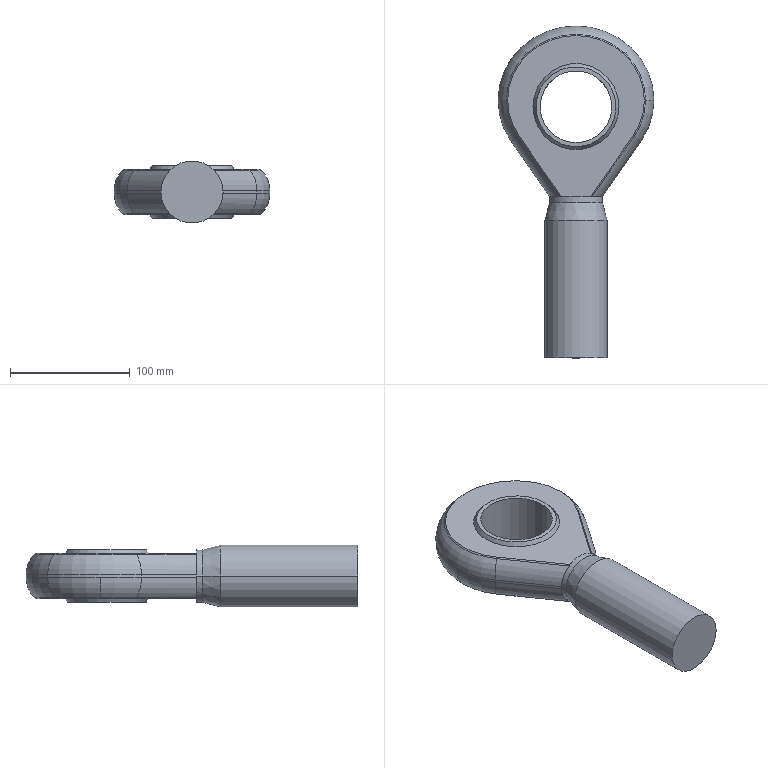Part | SolidWorks | features BaseBody 1 | 1 solid | 55 faces | box 130.224 x 277.5 x 52 mm | volume 678735 mm3 | cylinder 18 | plane 17 | cone 10 | torus 8 | sphere 2 | commonest cylinder face diameters 48 x4 72 x4 120 x3 44 x2 52 x2 60 x2
STEP:
#1=CARTESIAN_POINT('',(-65.112,5.488,-1.059));
#2=VERTEX_POINT('',#1);
#3=CARTESIAN_POINT('',(-54.261,-28.927,-1.059));
#4=VERTEX_POINT('',#3);
#5=CARTESIAN_POINT('',(-5.112,5.488,-1.059));
#6=DIRECTION('',(0.,0.,1.));
#7=DIRECTION('',(-1.,0.,0.));
#8=AXIS2_PLACEMENT_3D('',#5,#6,#7);
#9=CIRCLE('',#8,60.);
#10=EDGE_CURVE('',#2,#4,#9,.T.);
#11=ORIENTED_EDGE('',*,*,#10,.F.);
#12=CARTESIAN_POINT('',(-58.082,5.488,-18.029));
#13=VERTEX_POINT('',#12);
#14=CARTESIAN_POINT('',(-41.112,5.488,-1.059));
#15=DIRECTION('',(0.,-1.,0.));
#16=DIRECTION('',(0.,0.,-1.));
#17=AXIS2_PLACEMENT_3D('',#14,#15,#16);
#18=CIRCLE('',#17,24.);
#19=EDGE_CURVE('',#2,#13,#18,.T.);
#20=ORIENTED_EDGE('',*,*,#19,.T.);
#21=CARTESIAN_POINT('',(-48.503,-24.895,-18.029));
#22=VERTEX_POINT('',#21);
#23=CARTESIAN_POINT('',(-5.112,5.488,-18.029));
#24=DIRECTION('',(0.,0.,-1.));
#25=DIRECTION('',(-1.,0.,0.));
#26=AXIS2_PLACEMENT_3D('',#23,#24,#25);
#27=CIRCLE('',#26,52.971);
#28=EDGE_CURVE('',#22,#13,#27,.T.);
#29=ORIENTED_EDGE('',*,*,#28,.F.);
#30=CARTESIAN_POINT('',(-34.601,-15.161,-1.059));
#31=DIRECTION('',(-0.5736,0.8192,0.));
#32=DIRECTION('',(-0.8192,-0.5736,0.));
#33=AXIS2_PLACEMENT_3D('',#30,#31,#32);
#34=CIRCLE('',#33,24.);
#35=EDGE_CURVE('',#22,#4,#34,.T.);
#36=ORIENTED_EDGE('',*,*,#35,.T.);
#37=EDGE_LOOP('',(#11,#20,#29,#36));
#38=FACE_OUTER_BOUND('',#37,.T.);
#39=CARTESIAN_POINT('',(-5.112,5.488,-1.059));
#40=DIRECTION('',(0.,0.,-1.));
#41=DIRECTION('',(-1.,0.,0.));
#42=AXIS2_PLACEMENT_3D('',#39,#40,#41);
#43=TOROIDAL_SURFACE('',#42,36.,24.);
#44=ADVANCED_FACE('',(#38),#43,.T.);
#45=CARTESIAN_POINT('',(65.112,5.488,1.059));
#46=VERTEX_POINT('',#45);
#47=CARTESIAN_POINT('',(54.261,-28.927,1.059));
#48=VERTEX_POINT('',#47);
#49=CARTESIAN_POINT('',(5.112,5.488,1.059));
#50=DIRECTION('',(0.,0.,-1.));
#51=DIRECTION('',(1.,0.,0.));
#52=AXIS2_PLACEMENT_3D('',#49,#50,#51);
#53=CIRCLE('',#52,60.);
#54=EDGE_CURVE('',#46,#48,#53,.T.);
#55=ORIENTED_EDGE('',*,*,#54,.F.);
#56=CARTESIAN_POINT('',(58.082,5.488,18.029));
#57=VERTEX_POINT('',#56);
#58=CARTESIAN_POINT('',(41.112,5.488,1.059));
#59=DIRECTION('',(0.,-1.,0.));
#60=DIRECTION('',(0.,0.,-1.));
#61=AXIS2_PLACEMENT_3D('',#58,#59,#60);
#62=CIRCLE('',#61,24.);
#63=EDGE_CURVE('',#46,#57,#62,.T.);
#64=ORIENTED_EDGE('',*,*,#63,.T.);
#65=CARTESIAN_POINT('',(48.503,-24.895,18.029));
#66=VERTEX_POINT('',#65);
#67=CARTESIAN_POINT('',(5.112,5.488,18.029));
#68=DIRECTION('',(0.,0.,1.));
#69=DIRECTION('',(1.,0.,0.));
#70=AXIS2_PLACEMENT_3D('',#67,#68,#69);
#71=CIRCLE('',#70,52.971);
#72=EDGE_CURVE('',#66,#57,#71,.T.);
#73=ORIENTED_EDGE('',*,*,#72,.F.);
#74=CARTESIAN_POINT('',(34.601,-15.161,1.059));
#75=DIRECTION('',(0.5736,0.8192,0.));
#76=DIRECTION('',(-0.8192,0.5736,0.));
#77=AXIS2_PLACEMENT_3D('',#74,#75,#76);
#78=CIRCLE('',#77,24.);
#79=EDGE_CURVE('',#66,#48,#78,.T.);
#80=ORIENTED_EDGE('',*,*,#79,.T.);
#81=EDGE_LOOP('',(#55,#64,#73,#80));
#82=FACE_OUTER_BOUND('',#81,.T.);
#83=CARTESIAN_POINT('',(5.112,5.488,1.059));
#84=DIRECTION('',(0.,0.,1.));
#85=DIRECTION('',(1.,0.,0.));
#86=AXIS2_PLACEMENT_3D('',#83,#84,#85);
#87=TOROIDAL_SURFACE('',#86,36.,24.);
#88=ADVANCED_FACE('',(#82),#87,.T.);
#89=CARTESIAN_POINT('',(57.112,5.488,-19.));
#90=VERTEX_POINT('',#89);
#91=CARTESIAN_POINT('',(47.708,-24.338,-19.));
#92=VERTEX_POINT('',#91);
#93=CARTESIAN_POINT('',(5.112,5.488,-19.));
#94=DIRECTION('',(0.,0.,-1.));
#95=DIRECTION('',(1.,0.,0.));
#96=AXIS2_PLACEMENT_3D('',#93,#94,#95);
#97=CIRCLE('',#96,52.);
#98=EDGE_CURVE('',#90,#92,#97,.T.);
#99=ORIENTED_EDGE('',*,*,#98,.F.);
#100=CARTESIAN_POINT('',(58.082,5.488,-18.029));
#101=VERTEX_POINT('',#100);
#102=CARTESIAN_POINT('',(57.112,5.488,-19.));
#103=DIRECTION('',(0.7071,0.,0.7071));
#104=VECTOR('',#103,1000.);
#105=LINE('',#102,#104);
#106=EDGE_CURVE('',#90,#101,#105,.T.);
#107=ORIENTED_EDGE('',*,*,#106,.T.);
#108=CARTESIAN_POINT('',(48.503,-24.895,-18.029));
#109=VERTEX_POINT('',#108);
#110=CARTESIAN_POINT('',(5.112,5.488,-18.029));
#111=DIRECTION('',(0.,0.,-1.));
#112=DIRECTION('',(-1.,0.,0.));
#113=AXIS2_PLACEMENT_3D('',#110,#111,#112);
#114=CIRCLE('',#113,52.971);
#115=EDGE_CURVE('',#101,#109,#114,.T.);
#116=ORIENTED_EDGE('',*,*,#115,.T.);
#117=CARTESIAN_POINT('',(47.708,-24.338,-19.));
#118=DIRECTION('',(0.5792,-0.4056,0.7071));
#119=VECTOR('',#118,1000.);
#120=LINE('',#117,#119);
#121=EDGE_CURVE('',#92,#109,#120,.T.);
#122=ORIENTED_EDGE('',*,*,#121,.F.);
#123=EDGE_LOOP('',(#99,#107,#116,#122));
#124=FACE_OUTER_BOUND('',#123,.T.);
#125=CARTESIAN_POINT('',(5.112,5.488,-19.));
#126=DIRECTION('',(0.,0.,1.));
#127=DIRECTION('',(1.,0.,0.));
#128=AXIS2_PLACEMENT_3D('',#125,#126,#127);
#129=CONICAL_SURFACE('',#128,52.,0.7854);
#130=ADVANCED_FACE('',(#124),#129,.T.);
#131=CARTESIAN_POINT('',(-57.112,5.488,19.));
#132=VERTEX_POINT('',#131);
#133=CARTESIAN_POINT('',(-47.708,-24.338,19.));
#134=VERTEX_POINT('',#133);
#135=CARTESIAN_POINT('',(-5.112,5.488,19.));
#136=DIRECTION('',(0.,0.,1.));
#137=DIRECTION('',(1.,0.,0.));
#138=AXIS2_PLACEMENT_3D('',#135,#136,#137);
#139=CIRCLE('',#138,52.);
#140=EDGE_CURVE('',#132,#134,#139,.T.);
#141=ORIENTED_EDGE('',*,*,#140,.F.);
#142=CARTESIAN_POINT('',(-58.082,5.488,18.029));
#143=VERTEX_POINT('',#142);
#144=CARTESIAN_POINT('',(-57.112,5.488,19.));
#145=DIRECTION('',(-0.7071,0.,-0.7071));
#146=VECTOR('',#145,1000.);
#147=LINE('',#144,#146);
#148=EDGE_CURVE('',#132,#143,#147,.T.);
#149=ORIENTED_EDGE('',*,*,#148,.T.);
#150=CARTESIAN_POINT('',(-48.503,-24.895,18.029));
#151=VERTEX_POINT('',#150);
#152=CARTESIAN_POINT('',(-5.112,5.488,18.029));
#153=DIRECTION('',(0.,0.,1.));
#154=DIRECTION('',(1.,0.,0.));
#155=AXIS2_PLACEMENT_3D('',#152,#153,#154);
#156=CIRCLE('',#155,52.971);
#157=EDGE_CURVE('',#143,#151,#156,.T.);
#158=ORIENTED_EDGE('',*,*,#157,.T.);
#159=CARTESIAN_POINT('',(-54.261,-28.927,11.));
#160=DIRECTION('',(0.5792,0.4056,0.7071));
#161=VECTOR('',#160,1000.);
#162=LINE('',#159,#161);
#163=EDGE_CURVE('',#151,#134,#162,.T.);
#164=ORIENTED_EDGE('',*,*,#163,.T.);
#165=EDGE_LOOP('',(#141,#149,#158,#164));
#166=FACE_OUTER_BOUND('',#165,.T.);
#167=CARTESIAN_POINT('',(-5.112,5.488,19.));
#168=DIRECTION('',(0.,0.,-1.));
#169=DIRECTION('',(-1.,0.,0.));
#170=AXIS2_PLACEMENT_3D('',#167,#168,#169);
#171=CONICAL_SURFACE('',#170,52.,0.7854);
#172=ADVANCED_FACE('',(#166),#171,.T.);
#173=CARTESIAN_POINT('',(-22.,-80.072,0.));
#174=VERTEX_POINT('',#173);
#175=CARTESIAN_POINT('',(22.,-80.072,0.));
#176=VERTEX_POINT('',#175);
#177=CARTESIAN_POINT('',(0.,-80.072,0.));
#178=DIRECTION('',(0.,1.,0.));
#179=DIRECTION('',(-1.,0.,0.));
#180=AXIS2_PLACEMENT_3D('',#177,#178,#179);
#181=CIRCLE('',#180,22.);
#182=EDGE_CURVE('',#174,#176,#181,.T.);
#183=ORIENTED_EDGE('',*,*,#182,.F.);
#184=CARTESIAN_POINT('',(-26.,-95.,0.));
#185=VERTEX_POINT('',#184);
#186=CARTESIAN_POINT('',(-22.,-80.072,0.));
#187=DIRECTION('',(-0.2588,-0.9659,0.));
#188=VECTOR('',#187,1000.);
#189=LINE('',#186,#188);
#190=EDGE_CURVE('',#174,#185,#189,.T.);
#191=ORIENTED_EDGE('',*,*,#190,.T.);
#192=CARTESIAN_POINT('',(26.,-95.,0.));
#193=VERTEX_POINT('',#192);
#194=CARTESIAN_POINT('',(0.,-95.,0.));
#195=DIRECTION('',(0.,1.,0.));
#196=DIRECTION('',(-1.,0.,0.));
#197=AXIS2_PLACEMENT_3D('',#194,#195,#196);
#198=CIRCLE('',#197,26.);
#199=EDGE_CURVE('',#185,#193,#198,.T.);
#200=ORIENTED_EDGE('',*,*,#199,.T.);
#201=CARTESIAN_POINT('',(22.,-80.072,0.));
#202=DIRECTION('',(0.2588,-0.9659,0.));
#203=VECTOR('',#202,1000.);
#204=LINE('',#201,#203);
#205=EDGE_CURVE('',#176,#193,#204,.T.);
#206=ORIENTED_EDGE('',*,*,#205,.F.);
#207=EDGE_LOOP('',(#183,#191,#200,#206));
#208=FACE_OUTER_BOUND('',#207,.T.);
#209=CARTESIAN_POINT('',(0.,-80.072,0.));
#210=DIRECTION('',(0.,-1.,0.));
#211=DIRECTION('',(1.,0.,0.));
#212=AXIS2_PLACEMENT_3D('',#209,#210,#211);
#213=CONICAL_SURFACE('',#212,22.,0.2618);
#214=ADVANCED_FACE('',(#208),#213,.T.);
#215=CARTESIAN_POINT('',(26.,-210.,0.));
#216=VERTEX_POINT('',#215);
#217=CARTESIAN_POINT('',(-26.,-210.,0.));
#218=VERTEX_POINT('',#217);
#219=CARTESIAN_POINT('',(0.,-210.,0.));
#220=DIRECTION('',(0.,-1.,0.));
#221=DIRECTION('',(1.,0.,0.));
#222=AXIS2_PLACEMENT_3D('',#219,#220,#221);
#223=CIRCLE('',#222,26.);
#224=EDGE_CURVE('',#216,#218,#223,.T.);
#225=ORIENTED_EDGE('',*,*,#224,.F.);
#226=CARTESIAN_POINT('',(26.,-210.,0.));
#227=DIRECTION('',(0.,1.,0.));
#228=VECTOR('',#227,1000.);
#229=LINE('',#226,#228);
#230=EDGE_CURVE('',#216,#193,#229,.T.);
#231=ORIENTED_EDGE('',*,*,#230,.T.);
#232=ORIENTED_EDGE('',*,*,#199,.F.);
#233=CARTESIAN_POINT('',(-26.,-210.,0.));
#234=DIRECTION('',(0.,1.,0.));
#235=VECTOR('',#234,1000.);
#236=LINE('',#233,#235);
#237=EDGE_CURVE('',#218,#185,#236,.T.);
#238=ORIENTED_EDGE('',*,*,#237,.F.);
#239=EDGE_LOOP('',(#225,#231,#232,#238));
#240=FACE_OUTER_BOUND('',#239,.T.);
#241=CARTESIAN_POINT('',(0.,-210.,0.));
#242=DIRECTION('',(0.,1.,0.));
#243=DIRECTION('',(-1.,0.,0.));
#244=AXIS2_PLACEMENT_3D('',#241,#242,#243);
#245=CYLINDRICAL_SURFACE('',#244,26.);
#246=ADVANCED_FACE('',(#240),#245,.T.);
#247=ORIENTED_EDGE('',*,*,#182,.T.);
#248=CARTESIAN_POINT('',(22.,-75.,0.));
#249=VERTEX_POINT('',#248);
#250=CARTESIAN_POINT('',(22.,-95.,0.));
#251=DIRECTION('',(0.,1.,0.));
#252=VECTOR('',#251,1000.);
#253=LINE('',#250,#252);
#254=EDGE_CURVE('',#176,#249,#253,.T.);
#255=ORIENTED_EDGE('',*,*,#254,.T.);
#256=CARTESIAN_POINT('',(11.091,-75.,19.));
#257=VERTEX_POINT('',#256);
#258=CARTESIAN_POINT('',(0.,-75.,0.));
#259=DIRECTION('',(0.,1.,0.));
#260=DIRECTION('',(-1.,0.,0.));
#261=AXIS2_PLACEMENT_3D('',#258,#259,#260);
#262=CIRCLE('',#261,22.);
#263=EDGE_CURVE('',#257,#249,#262,.T.);
#264=ORIENTED_EDGE('',*,*,#263,.F.);
#265=CARTESIAN_POINT('',(-11.091,-75.,19.));
#266=VERTEX_POINT('',#265);
#267=CARTESIAN_POINT('',(0.,-75.,0.));
#268=DIRECTION('',(0.,1.,0.));
#269=DIRECTION('',(-1.,0.,0.));
#270=AXIS2_PLACEMENT_3D('',#267,#268,#269);
#271=CIRCLE('',#270,22.);
#272=EDGE_CURVE('',#266,#257,#271,.T.);
#273=ORIENTED_EDGE('',*,*,#272,.F.);
#274=CARTESIAN_POINT('',(-22.,-75.,0.));
#275=VERTEX_POINT('',#274);
#276=CARTESIAN_POINT('',(0.,-75.,0.));
#277=DIRECTION('',(0.,1.,0.));
#278=DIRECTION('',(-1.,0.,0.));
#279=AXIS2_PLACEMENT_3D('',#276,#277,#278);
#280=CIRCLE('',#279,22.);
#281=EDGE_CURVE('',#275,#266,#280,.T.);
#282=ORIENTED_EDGE('',*,*,#281,.F.);
#283=CARTESIAN_POINT('',(-22.,-95.,0.));
#284=DIRECTION('',(0.,1.,0.));
#285=VECTOR('',#284,1000.);
#286=LINE('',#283,#285);
#287=EDGE_CURVE('',#174,#275,#286,.T.);
#288=ORIENTED_EDGE('',*,*,#287,.F.);
#289=EDGE_LOOP('',(#247,#255,#264,#273,#282,#288));
#290=FACE_OUTER_BOUND('',#289,.T.);
#291=CARTESIAN_POINT('',(0.,-95.,0.));
#292=DIRECTION('',(0.,1.,0.));
#293=DIRECTION('',(-1.,0.,0.));
#294=AXIS2_PLACEMENT_3D('',#291,#292,#293);
#295=CYLINDRICAL_SURFACE('',#294,22.);
#296=ADVANCED_FACE('',(#290),#295,.T.);
#297=CARTESIAN_POINT('',(54.261,-28.927,-1.059));
#298=VERTEX_POINT('',#297);
#299=CARTESIAN_POINT('',(65.112,5.488,-1.059));
#300=VERTEX_POINT('',#299);
#301=CARTESIAN_POINT('',(5.112,5.488,-1.059));
#302=DIRECTION('',(0.,0.,1.));
#303=DIRECTION('',(-1.,0.,0.));
#304=AXIS2_PLACEMENT_3D('',#301,#302,#303);
#305=CIRCLE('',#304,60.);
#306=EDGE_CURVE('',#298,#300,#305,.T.);
#307=ORIENTED_EDGE('',*,*,#306,.T.);
#308=CARTESIAN_POINT('',(65.112,5.488,-19.));
#309=DIRECTION('',(0.,0.,1.));
#310=VECTOR('',#309,1000.);
#311=LINE('',#308,#310);
#312=EDGE_CURVE('',#300,#46,#311,.T.);
#313=ORIENTED_EDGE('',*,*,#312,.T.);
#314=ORIENTED_EDGE('',*,*,#54,.T.);
#315=CARTESIAN_POINT('',(54.261,-28.927,19.));
#316=DIRECTION('',(0.,0.,1.));
#317=VECTOR('',#316,1000.);
#318=LINE('',#315,#317);
#319=EDGE_CURVE('',#298,#48,#318,.T.);
#320=ORIENTED_EDGE('',*,*,#319,.F.);
#321=EDGE_LOOP('',(#307,#313,#314,#320));
#322=FACE_OUTER_BOUND('',#321,.T.);
#323=CARTESIAN_POINT('',(5.112,5.488,-19.));
#324=DIRECTION('',(0.,0.,1.));
#325=DIRECTION('',(1.,0.,0.));
#326=AXIS2_PLACEMENT_3D('',#323,#324,#325);
#327=CYLINDRICAL_SURFACE('',#326,60.);
#328=ADVANCED_FACE('',(#322),#327,.T.);
#329=CARTESIAN_POINT('',(36.,0.,-19.));
#330=VERTEX_POINT('',#329);
#331=CARTESIAN_POINT('',(-36.,0.,-19.));
#332=VERTEX_POINT('',#331);
#333=CARTESIAN_POINT('',(0.,0.,-19.));
#334=DIRECTION('',(0.,0.,-1.));
#335=DIRECTION('',(1.,0.,0.));
#336=AXIS2_PLACEMENT_3D('',#333,#334,#335);
#337=CIRCLE('',#336,36.);
#338=EDGE_CURVE('',#330,#332,#337,.T.);
#339=ORIENTED_EDGE('',*,*,#338,.T.);
#340=CARTESIAN_POINT('',(-36.,0.,-17.436));
#341=VERTEX_POINT('',#340);
#342=CARTESIAN_POINT('',(-36.,0.,-19.));
#343=DIRECTION('',(0.,0.,1.));
#344=VECTOR('',#343,1000.);
#345=LINE('',#342,#344);
#346=EDGE_CURVE('',#332,#341,#345,.T.);
#347=ORIENTED_EDGE('',*,*,#346,.T.);
#348=CARTESIAN_POINT('',(36.,0.,-17.436));
#349=VERTEX_POINT('',#348);
#350=CARTESIAN_POINT('',(0.,0.,-17.436));
#351=DIRECTION('',(0.,0.,1.));
#352=DIRECTION('',(1.,0.,0.));
#353=AXIS2_PLACEMENT_3D('',#350,#351,#352);
#354=CIRCLE('',#353,36.);
#355=EDGE_CURVE('',#341,#349,#354,.T.);
#356=ORIENTED_EDGE('',*,*,#355,.T.);
#357=CARTESIAN_POINT('',(36.,0.,-19.));
#358=DIRECTION('',(0.,0.,1.));
#359=VECTOR('',#358,1000.);
#360=LINE('',#357,#359);
#361=EDGE_CURVE('',#330,#349,#360,.T.);
#362=ORIENTED_EDGE('',*,*,#361,.F.);
#363=EDGE_LOOP('',(#339,#347,#356,#362));
#364=FACE_OUTER_BOUND('',#363,.T.);
#365=CARTESIAN_POINT('',(0.,0.,-19.));
#366=DIRECTION('',(0.,0.,1.));
#367=DIRECTION('',(1.,0.,0.));
#368=AXIS2_PLACEMENT_3D('',#365,#366,#367);
#369=CYLINDRICAL_SURFACE('',#368,36.);
#370=ADVANCED_FACE('',(#364),#369,.F.);
#371=CARTESIAN_POINT('',(36.,0.,17.436));
#372=VERTEX_POINT('',#371);
#373=CARTESIAN_POINT('',(-36.,0.,17.436));
#374=VERTEX_POINT('',#373);
#375=CARTESIAN_POINT('',(0.,0.,17.436));
#376=DIRECTION('',(0.,0.,-1.));
#377=DIRECTION('',(-1.,0.,0.));
#378=AXIS2_PLACEMENT_3D('',#375,#376,#377);
#379=CIRCLE('',#378,36.);
#380=EDGE_CURVE('',#372,#374,#379,.T.);
#381=ORIENTED_EDGE('',*,*,#380,.T.);
#382=CARTESIAN_POINT('',(-36.,0.,19.));
#383=VERTEX_POINT('',#382);
#384=CARTESIAN_POINT('',(-36.,0.,-19.));
#385=DIRECTION('',(0.,0.,1.));
#386=VECTOR('',#385,1000.);
#387=LINE('',#384,#386);
#388=EDGE_CURVE('',#374,#383,#387,.T.);
#389=ORIENTED_EDGE('',*,*,#388,.T.);
#390=CARTESIAN_POINT('',(36.,0.,19.));
#391=VERTEX_POINT('',#390);
#392=CARTESIAN_POINT('',(0.,0.,19.));
#393=DIRECTION('',(0.,0.,-1.));
#394=DIRECTION('',(1.,0.,0.));
#395=AXIS2_PLACEMENT_3D('',#392,#393,#394);
#396=CIRCLE('',#395,36.);
#397=EDGE_CURVE('',#391,#383,#396,.T.);
#398=ORIENTED_EDGE('',*,*,#397,.F.);
#399=CARTESIAN_POINT('',(36.,0.,-19.));
#400=DIRECTION('',(0.,0.,1.));
#401=VECTOR('',#400,1000.);
#402=LINE('',#399,#401);
#403=EDGE_CURVE('',#372,#391,#402,.T.);
#404=ORIENTED_EDGE('',*,*,#403,.F.);
#405=EDGE_LOOP('',(#381,#389,#398,#404));
#406=FACE_OUTER_BOUND('',#405,.T.);
#407=CARTESIAN_POINT('',(0.,0.,-19.));
#408=DIRECTION('',(0.,0.,1.));
#409=DIRECTION('',(1.,0.,0.));
#410=AXIS2_PLACEMENT_3D('',#407,#408,#409);
#411=CYLINDRICAL_SURFACE('',#410,36.);
#412=ADVANCED_FACE('',(#406),#411,.F.);
#413=CARTESIAN_POINT('',(-30.,0.,22.));
#414=VERTEX_POINT('',#413);
#415=CARTESIAN_POINT('',(30.,0.,22.));
#416=VERTEX_POINT('',#415);
#417=CARTESIAN_POINT('',(0.,0.,22.));
#418=DIRECTION('',(0.,0.,1.));
#419=DIRECTION('',(-1.,0.,0.));
#420=AXIS2_PLACEMENT_3D('',#417,#418,#419);
#421=CIRCLE('',#420,30.);
#422=EDGE_CURVE('',#414,#416,#421,.T.);
#423=ORIENTED_EDGE('',*,*,#422,.T.);
#424=CARTESIAN_POINT('',(30.,0.,-22.));
#425=VERTEX_POINT('',#424);
#426=CARTESIAN_POINT('',(30.,0.,63.));
#427=DIRECTION('',(0.,0.,-1.));
#428=VECTOR('',#427,1000.);
#429=LINE('',#426,#428);
#430=EDGE_CURVE('',#416,#425,#429,.T.);
#431=ORIENTED_EDGE('',*,*,#430,.T.);
#432=CARTESIAN_POINT('',(-30.,0.,-22.));
#433=VERTEX_POINT('',#432);
#434=CARTESIAN_POINT('',(0.,0.,-22.));
#435=DIRECTION('',(0.,0.,-1.));
#436=DIRECTION('',(1.,0.,0.));
#437=AXIS2_PLACEMENT_3D('',#434,#435,#436);
#438=CIRCLE('',#437,30.);
#439=EDGE_CURVE('',#425,#433,#438,.T.);
#440=ORIENTED_EDGE('',*,*,#439,.T.);
#441=CARTESIAN_POINT('',(-30.,0.,63.));
#442=DIRECTION('',(0.,0.,-1.));
#443=VECTOR('',#442,1000.);
#444=LINE('',#441,#443);
#445=EDGE_CURVE('',#414,#433,#444,.T.);
#446=ORIENTED_EDGE('',*,*,#445,.F.);
#447=EDGE_LOOP('',(#423,#431,#440,#446));
#448=FACE_OUTER_BOUND('',#447,.T.);
#449=CARTESIAN_POINT('',(0.,0.,63.));
#450=DIRECTION('',(0.,0.,-1.));
#451=DIRECTION('',(-1.,0.,0.));
#452=AXIS2_PLACEMENT_3D('',#449,#450,#451);
#453=CYLINDRICAL_SURFACE('',#452,30.);
#454=ADVANCED_FACE('',(#448),#453,.F.);
#455=CARTESIAN_POINT('',(11.091,-75.,-19.));
#456=VERTEX_POINT('',#455);
#457=CARTESIAN_POINT('',(-11.091,-75.,-19.));
#458=VERTEX_POINT('',#457);
#459=CARTESIAN_POINT('',(0.,-75.,0.));
#460=DIRECTION('',(0.,1.,0.));
#461=DIRECTION('',(-1.,0.,0.));
#462=AXIS2_PLACEMENT_3D('',#459,#460,#461);
#463=CIRCLE('',#462,22.);
#464=EDGE_CURVE('',#456,#458,#463,.T.);
#465=ORIENTED_EDGE('',*,*,#464,.T.);
#466=CARTESIAN_POINT('',(-22.,-75.,-19.));
#467=DIRECTION('',(1.,0.,0.));
#468=VECTOR('',#467,1000.);
#469=LINE('',#466,#468);
#470=EDGE_CURVE('',#458,#456,#469,.T.);
#471=ORIENTED_EDGE('',*,*,#470,.T.);
#472=EDGE_LOOP('',(#465,#471));
#473=FACE_OUTER_BOUND('',#472,.T.);
#474=CARTESIAN_POINT('',(0.,-75.,0.));
#475=DIRECTION('',(0.,-1.,0.));
#476=DIRECTION('',(1.,0.,0.));
#477=AXIS2_PLACEMENT_3D('',#474,#475,#476);
#478=PLANE('',#477);
#479=ADVANCED_FACE('',(#473),#478,.F.);
#480=ORIENTED_EDGE('',*,*,#272,.T.);
#481=CARTESIAN_POINT('',(-22.,-75.,19.));
#482=DIRECTION('',(1.,0.,0.));
#483=VECTOR('',#482,1000.);
#484=LINE('',#481,#483);
#485=EDGE_CURVE('',#266,#257,#484,.T.);
#486=ORIENTED_EDGE('',*,*,#485,.F.);
#487=EDGE_LOOP('',(#480,#486));
#488=FACE_OUTER_BOUND('',#487,.T.);
#489=CARTESIAN_POINT('',(0.,-75.,0.));
#490=DIRECTION('',(0.,-1.,0.));
#491=DIRECTION('',(1.,0.,0.));
#492=AXIS2_PLACEMENT_3D('',#489,#490,#491);
#493=PLANE('',#492);
#494=ADVANCED_FACE('',(#488),#493,.F.);
#495=CARTESIAN_POINT('',(22.,-75.,1.059));
#496=VERTEX_POINT('',#495);
#497=CARTESIAN_POINT('',(22.,-75.,-19.));
#498=DIRECTION('',(0.,0.,1.));
#499=VECTOR('',#498,1000.);
#500=LINE('',#497,#499);
#501=EDGE_CURVE('',#249,#496,#500,.T.);
#502=ORIENTED_EDGE('',*,*,#501,.T.);
#503=CARTESIAN_POINT('',(13.419,-75.,18.029));
#504=VERTEX_POINT('',#503);
#505=CARTESIAN_POINT('',(22.,-75.,1.059));
#506=CARTESIAN_POINT('',(22.,-75.,7.509));
#507=CARTESIAN_POINT('',(18.987,-75.,13.468));
#508=CARTESIAN_POINT('',(13.419,-75.,18.029));
#509=(BOUNDED_CURVE()B_SPLINE_CURVE(3,(#505,#506,#507,#508),.UNSPECIFIED.,.F.,.F.)B_SPLINE_CURVE_WITH_KNOTS((4,4),(0.,0.7854),.UNSPECIFIED.)CURVE()GEOMETRIC_REPRESENTATION_ITEM()RATIONAL_B_SPLINE_CURVE((1.,0.9493,0.9493,1.))REPRESENTATION_ITEM(''));
#510=EDGE_CURVE('',#496,#504,#509,.T.);
#511=ORIENTED_EDGE('',*,*,#510,.T.);
#512=CARTESIAN_POINT('',(12.234,-75.,19.));
#513=VERTEX_POINT('',#512);
#514=CARTESIAN_POINT('',(10.375,-75.,20.523));
#515=DIRECTION('',(-0.7736,0.,0.6337));
#516=VECTOR('',#515,1000.);
#517=LINE('',#514,#516);
#518=EDGE_CURVE('',#504,#513,#517,.T.);
#519=ORIENTED_EDGE('',*,*,#518,.T.);
#520=CARTESIAN_POINT('',(-22.,-75.,19.));
#521=DIRECTION('',(1.,0.,0.));
#522=VECTOR('',#521,1000.);
#523=LINE('',#520,#522);
#524=EDGE_CURVE('',#257,#513,#523,.T.);
#525=ORIENTED_EDGE('',*,*,#524,.F.);
#526=ORIENTED_EDGE('',*,*,#263,.T.);
#527=EDGE_LOOP('',(#502,#511,#519,#525,#526));
#528=FACE_OUTER_BOUND('',#527,.T.);
#529=CARTESIAN_POINT('',(-22.,-75.,-19.));
#530=DIRECTION('',(0.,-1.,0.));
#531=DIRECTION('',(1.,0.,0.));
#532=AXIS2_PLACEMENT_3D('',#529,#530,#531);
#533=PLANE('',#532);
#534=ADVANCED_FACE('',(#528),#533,.T.);
#535=CARTESIAN_POINT('',(-12.234,-75.,19.));
#536=VERTEX_POINT('',#535);
#537=CARTESIAN_POINT('',(-13.419,-75.,18.029));
#538=VERTEX_POINT('',#537);
#539=CARTESIAN_POINT('',(-36.706,-75.,-1.047));
#540=DIRECTION('',(-0.7736,0.,-0.6337));
#541=VECTOR('',#540,1000.);
#542=LINE('',#539,#541);
#543=EDGE_CURVE('',#536,#538,#542,.T.);
#544=ORIENTED_EDGE('',*,*,#543,.T.);
#545=CARTESIAN_POINT('',(-22.,-75.,1.059));
#546=VERTEX_POINT('',#545);
#547=CARTESIAN_POINT('',(-13.419,-75.,18.029));
#548=CARTESIAN_POINT('',(-18.987,-75.,13.468));
#549=CARTESIAN_POINT('',(-22.,-75.,7.509));
#550=CARTESIAN_POINT('',(-22.,-75.,1.059));
#551=(BOUNDED_CURVE()B_SPLINE_CURVE(3,(#547,#548,#549,#550),.UNSPECIFIED.,.F.,.F.)B_SPLINE_CURVE_WITH_KNOTS((4,4),(2.356,3.142),.UNSPECIFIED.)CURVE()GEOMETRIC_REPRESENTATION_ITEM()RATIONAL_B_SPLINE_CURVE((1.,0.9493,0.9493,1.))REPRESENTATION_ITEM(''));
#552=EDGE_CURVE('',#538,#546,#551,.T.);
#553=ORIENTED_EDGE('',*,*,#552,.T.);
#554=CARTESIAN_POINT('',(-22.,-75.,-19.));
#555=DIRECTION('',(0.,0.,1.));
#556=VECTOR('',#555,1000.);
#557=LINE('',#554,#556);
#558=EDGE_CURVE('',#275,#546,#557,.T.);
#559=ORIENTED_EDGE('',*,*,#558,.F.);
#560=ORIENTED_EDGE('',*,*,#281,.T.);
#561=CARTESIAN_POINT('',(-22.,-75.,19.));
#562=DIRECTION('',(1.,0.,0.));
#563=VECTOR('',#562,1000.);
#564=LINE('',#561,#563);
#565=EDGE_CURVE('',#536,#266,#564,.T.);
#566=ORIENTED_EDGE('',*,*,#565,.F.);
#567=EDGE_LOOP('',(#544,#553,#559,#560,#566));
#568=FACE_OUTER_BOUND('',#567,.T.);
#569=CARTESIAN_POINT('',(-22.,-75.,-19.));
#570=DIRECTION('',(0.,-1.,0.));
#571=DIRECTION('',(1.,0.,0.));
#572=AXIS2_PLACEMENT_3D('',#569,#570,#571);
#573=PLANE('',#572);
#574=ADVANCED_FACE('',(#568),#573,.T.);
#575=CARTESIAN_POINT('',(-22.,-75.,-1.059));
#576=VERTEX_POINT('',#575);
#577=CARTESIAN_POINT('',(-22.,-75.,-19.));
#578=DIRECTION('',(0.,0.,1.));
#579=VECTOR('',#578,1000.);
#580=LINE('',#577,#579);
#581=EDGE_CURVE('',#576,#275,#580,.T.);
#582=ORIENTED_EDGE('',*,*,#581,.F.);
#583=CARTESIAN_POINT('',(-13.419,-75.,-18.029));
#584=VERTEX_POINT('',#583);
#585=CARTESIAN_POINT('',(-22.,-75.,-1.059));
#586=CARTESIAN_POINT('',(-22.,-75.,-7.509));
#587=CARTESIAN_POINT('',(-18.987,-75.,-13.468));
#588=CARTESIAN_POINT('',(-13.419,-75.,-18.029));
#589=(BOUNDED_CURVE()B_SPLINE_CURVE(3,(#585,#586,#587,#588),.UNSPECIFIED.,.F.,.T.)B_SPLINE_CURVE_WITH_KNOTS((4,4),(3.142,3.927),.UNSPECIFIED.)CURVE()GEOMETRIC_REPRESENTATION_ITEM()RATIONAL_B_SPLINE_CURVE((1.,0.9493,0.9493,1.))REPRESENTATION_ITEM(''));
#590=EDGE_CURVE('',#576,#584,#589,.T.);
#591=ORIENTED_EDGE('',*,*,#590,.T.);
#592=CARTESIAN_POINT('',(-12.234,-75.,-19.));
#593=VERTEX_POINT('',#592);
#594=CARTESIAN_POINT('',(-18.078,-75.,-14.212));
#595=DIRECTION('',(0.7736,0.,-0.6337));
#596=VECTOR('',#595,1000.);
#597=LINE('',#594,#596);
#598=EDGE_CURVE('',#584,#593,#597,.T.);
#599=ORIENTED_EDGE('',*,*,#598,.T.);
#600=CARTESIAN_POINT('',(-22.,-75.,-19.));
#601=DIRECTION('',(1.,0.,0.));
#602=VECTOR('',#601,1000.);
#603=LINE('',#600,#602);
#604=EDGE_CURVE('',#593,#458,#603,.T.);
#605=ORIENTED_EDGE('',*,*,#604,.T.);
#606=CARTESIAN_POINT('',(0.,-75.,0.));
#607=DIRECTION('',(0.,1.,0.));
#608=DIRECTION('',(-1.,0.,0.));
#609=AXIS2_PLACEMENT_3D('',#606,#607,#608);
#610=CIRCLE('',#609,22.);
#611=EDGE_CURVE('',#458,#275,#610,.T.);
#612=ORIENTED_EDGE('',*,*,#611,.T.);
#613=EDGE_LOOP('',(#582,#591,#599,#605,#612));
#614=FACE_OUTER_BOUND('',#613,.T.);
#615=CARTESIAN_POINT('',(-22.,-75.,-19.));
#616=DIRECTION('',(0.,-1.,0.));
#617=DIRECTION('',(1.,0.,0.));
#618=AXIS2_PLACEMENT_3D('',#615,#616,#617);
#619=PLANE('',#618);
#620=ADVANCED_FACE('',(#614),#619,.T.);
#621=CARTESIAN_POINT('',(-33.407,0.,22.));
#622=VERTEX_POINT('',#621);
#623=CARTESIAN_POINT('',(33.407,0.,22.));
#624=VERTEX_POINT('',#623);
#625=CARTESIAN_POINT('',(0.,0.,22.));
#626=DIRECTION('',(0.,0.,1.));
#627=DIRECTION('',(-1.,0.,0.));
#628=AXIS2_PLACEMENT_3D('',#625,#626,#627);
#629=CIRCLE('',#628,33.407);
#630=EDGE_CURVE('',#622,#624,#629,.T.);
#631=ORIENTED_EDGE('',*,*,#630,.F.);
#632=CARTESIAN_POINT('',(0.,0.,22.));
#633=DIRECTION('',(0.,0.,1.));
#634=DIRECTION('',(-1.,0.,0.));
#635=AXIS2_PLACEMENT_3D('',#632,#633,#634);
#636=CIRCLE('',#635,33.407);
#637=EDGE_CURVE('',#624,#622,#636,.T.);
#638=ORIENTED_EDGE('',*,*,#637,.F.);
#639=EDGE_LOOP('',(#631,#638));
#640=FACE_BOUND('',#639,.T.);
#641=ORIENTED_EDGE('',*,*,#380,.F.);
#642=CARTESIAN_POINT('',(0.,0.,17.436));
#643=DIRECTION('',(0.,0.,-1.));
#644=DIRECTION('',(-1.,0.,0.));
#645=AXIS2_PLACEMENT_3D('',#642,#643,#644);
#646=CIRCLE('',#645,36.);
#647=EDGE_CURVE('',#374,#372,#646,.T.);
#648=ORIENTED_EDGE('',*,*,#647,.F.);
#649=EDGE_LOOP('',(#641,#648));
#650=FACE_OUTER_BOUND('',#649,.T.);
#651=CARTESIAN_POINT('',(0.,0.,0.));
#652=DIRECTION('',(0.,0.,-1.));
#653=DIRECTION('',(1.,0.,0.));
#654=AXIS2_PLACEMENT_3D('',#651,#652,#653);
#655=SPHERICAL_SURFACE('',#654,40.);
#656=ADVANCED_FACE('',(#640,#650),#655,.T.);
#657=CARTESIAN_POINT('',(33.407,0.,-22.));
#658=VERTEX_POINT('',#657);
#659=CARTESIAN_POINT('',(-33.407,0.,-22.));
#660=VERTEX_POINT('',#659);
#661=CARTESIAN_POINT('',(0.,0.,-22.));
#662=DIRECTION('',(0.,0.,-1.));
#663=DIRECTION('',(1.,0.,0.));
#664=AXIS2_PLACEMENT_3D('',#661,#662,#663);
#665=CIRCLE('',#664,33.407);
#666=EDGE_CURVE('',#658,#660,#665,.T.);
#667=ORIENTED_EDGE('',*,*,#666,.F.);
#668=CARTESIAN_POINT('',(0.,0.,-22.));
#669=DIRECTION('',(0.,0.,-1.));
#670=DIRECTION('',(1.,0.,0.));
#671=AXIS2_PLACEMENT_3D('',#668,#669,#670);
#672=CIRCLE('',#671,33.407);
#673=EDGE_CURVE('',#660,#658,#672,.T.);
#674=ORIENTED_EDGE('',*,*,#673,.F.);
#675=EDGE_LOOP('',(#667,#674));
#676=FACE_BOUND('',#675,.T.);
#677=CARTESIAN_POINT('',(0.,0.,-17.436));
#678=DIRECTION('',(0.,0.,1.));
#679=DIRECTION('',(1.,0.,0.));
#680=AXIS2_PLACEMENT_3D('',#677,#678,#679);
#681=CIRCLE('',#680,36.);
#682=EDGE_CURVE('',#349,#341,#681,.T.);
#683=ORIENTED_EDGE('',*,*,#682,.F.);
#684=ORIENTED_EDGE('',*,*,#355,.F.);
#685=EDGE_LOOP('',(#683,#684));
#686=FACE_OUTER_BOUND('',#685,.T.);
#687=CARTESIAN_POINT('',(0.,0.,0.));
#688=DIRECTION('',(0.,0.,-1.));
#689=DIRECTION('',(1.,0.,0.));
#690=AXIS2_PLACEMENT_3D('',#687,#688,#689);
#691=SPHERICAL_SURFACE('',#690,40.);
#692=ADVANCED_FACE('',(#676,#686),#691,.T.);
#693=CARTESIAN_POINT('',(0.,0.,-22.));
#694=DIRECTION('',(0.,0.,-1.));
#695=DIRECTION('',(1.,0.,0.));
#696=AXIS2_PLACEMENT_3D('',#693,#694,#695);
#697=CIRCLE('',#696,30.);
#698=EDGE_CURVE('',#433,#425,#697,.T.);
#699=ORIENTED_EDGE('',*,*,#698,.F.);
#700=ORIENTED_EDGE('',*,*,#439,.F.);
#701=EDGE_LOOP('',(#699,#700));
#702=FACE_BOUND('',#701,.T.);
#703=ORIENTED_EDGE('',*,*,#666,.T.);
#704=ORIENTED_EDGE('',*,*,#673,.T.);
#705=EDGE_LOOP('',(#703,#704));
#706=FACE_OUTER_BOUND('',#705,.T.);
#707=CARTESIAN_POINT('',(70.,-52.471,-22.));
#708=DIRECTION('',(0.,0.,1.));
#709=DIRECTION('',(1.,0.,0.));
#710=AXIS2_PLACEMENT_3D('',#707,#708,#709);
#711=PLANE('',#710);
#712=ADVANCED_FACE('',(#702,#706),#711,.F.);
#713=ORIENTED_EDGE('',*,*,#422,.F.);
#714=CARTESIAN_POINT('',(0.,0.,22.));
#715=DIRECTION('',(0.,0.,1.));
#716=DIRECTION('',(-1.,0.,0.));
#717=AXIS2_PLACEMENT_3D('',#714,#715,#716);
#718=CIRCLE('',#717,30.);
#719=EDGE_CURVE('',#416,#414,#718,.T.);
#720=ORIENTED_EDGE('',*,*,#719,.F.);
#721=EDGE_LOOP('',(#713,#720));
#722=FACE_BOUND('',#721,.T.);
#723=ORIENTED_EDGE('',*,*,#630,.T.);
#724=ORIENTED_EDGE('',*,*,#637,.T.);
#725=EDGE_LOOP('',(#723,#724));
#726=FACE_OUTER_BOUND('',#725,.T.);
#727=CARTESIAN_POINT('',(70.,-52.471,22.));
#728=DIRECTION('',(0.,0.,-1.));
#729=DIRECTION('',(-1.,0.,0.));
#730=AXIS2_PLACEMENT_3D('',#727,#728,#729);
#731=PLANE('',#730);
#732=ADVANCED_FACE('',(#722,#726),#731,.F.);
#733=ORIENTED_EDGE('',*,*,#430,.F.);
#734=ORIENTED_EDGE('',*,*,#719,.T.);
#735=ORIENTED_EDGE('',*,*,#445,.T.);
#736=ORIENTED_EDGE('',*,*,#698,.T.);
#737=EDGE_LOOP('',(#733,#734,#735,#736));
#738=FACE_OUTER_BOUND('',#737,.T.);
#739=CARTESIAN_POINT('',(0.,0.,63.));
#740=DIRECTION('',(0.,0.,-1.));
#741=DIRECTION('',(-1.,0.,0.));
#742=AXIS2_PLACEMENT_3D('',#739,#740,#741);
#743=CYLINDRICAL_SURFACE('',#742,30.);
#744=ADVANCED_FACE('',(#738),#743,.F.);
#745=ORIENTED_EDGE('',*,*,#388,.F.);
#746=ORIENTED_EDGE('',*,*,#647,.T.);
#747=ORIENTED_EDGE('',*,*,#403,.T.);
#748=CARTESIAN_POINT('',(0.,0.,19.));
#749=DIRECTION('',(0.,0.,-1.));
#750=DIRECTION('',(1.,0.,0.));
#751=AXIS2_PLACEMENT_3D('',#748,#749,#750);
#752=CIRCLE('',#751,36.);
#753=EDGE_CURVE('',#383,#391,#752,.T.);
#754=ORIENTED_EDGE('',*,*,#753,.F.);
#755=EDGE_LOOP('',(#745,#746,#747,#754));
#756=FACE_OUTER_BOUND('',#755,.T.);
#757=CARTESIAN_POINT('',(0.,0.,-19.));
#758=DIRECTION('',(0.,0.,1.));
#759=DIRECTION('',(1.,0.,0.));
#760=AXIS2_PLACEMENT_3D('',#757,#758,#759);
#761=CYLINDRICAL_SURFACE('',#760,36.);
#762=ADVANCED_FACE('',(#756),#761,.F.);
#763=CARTESIAN_POINT('',(-46.007,49.393,-1.059));
#764=VERTEX_POINT('',#763);
#765=CARTESIAN_POINT('',(-46.007,49.393,1.059));
#766=VERTEX_POINT('',#765);
#767=CARTESIAN_POINT('',(-46.007,49.393,-19.));
#768=DIRECTION('',(0.,0.,1.));
#769=VECTOR('',#768,1000.);
#770=LINE('',#767,#769);
#771=EDGE_CURVE('',#764,#766,#770,.T.);
#772=ORIENTED_EDGE('',*,*,#771,.T.);
#773=CARTESIAN_POINT('',(46.007,49.393,1.059));
#774=VERTEX_POINT('',#773);
#775=CARTESIAN_POINT('',(0.,0.,1.059));
#776=DIRECTION('',(0.,0.,-1.));
#777=DIRECTION('',(1.,0.,0.));
#778=AXIS2_PLACEMENT_3D('',#775,#776,#777);
#779=CIRCLE('',#778,67.5);
#780=EDGE_CURVE('',#766,#774,#779,.T.);
#781=ORIENTED_EDGE('',*,*,#780,.T.);
#782=CARTESIAN_POINT('',(46.007,49.393,-1.059));
#783=VERTEX_POINT('',#782);
#784=CARTESIAN_POINT('',(46.007,49.393,-19.));
#785=DIRECTION('',(0.,0.,-1.));
#786=VECTOR('',#785,1000.);
#787=LINE('',#784,#786);
#788=EDGE_CURVE('',#774,#783,#787,.T.);
#789=ORIENTED_EDGE('',*,*,#788,.T.);
#790=CARTESIAN_POINT('',(0.,0.,-1.059));
#791=DIRECTION('',(0.,0.,1.));
#792=DIRECTION('',(-1.,0.,0.));
#793=AXIS2_PLACEMENT_3D('',#790,#791,#792);
#794=CIRCLE('',#793,67.5);
#795=EDGE_CURVE('',#783,#764,#794,.T.);
#796=ORIENTED_EDGE('',*,*,#795,.T.);
#797=EDGE_LOOP('',(#772,#781,#789,#796));
#798=FACE_OUTER_BOUND('',#797,.T.);
#799=CARTESIAN_POINT('',(0.,0.,-19.));
#800=DIRECTION('',(0.,0.,1.));
#801=DIRECTION('',(1.,0.,0.));
#802=AXIS2_PLACEMENT_3D('',#799,#800,#801);
#803=CYLINDRICAL_SURFACE('',#802,67.5);
#804=ADVANCED_FACE('',(#798),#803,.T.);
#805=ORIENTED_EDGE('',*,*,#346,.F.);
#806=CARTESIAN_POINT('',(0.,0.,-19.));
#807=DIRECTION('',(0.,0.,-1.));
#808=DIRECTION('',(1.,0.,0.));
#809=AXIS2_PLACEMENT_3D('',#806,#807,#808);
#810=CIRCLE('',#809,36.);
#811=EDGE_CURVE('',#332,#330,#810,.T.);
#812=ORIENTED_EDGE('',*,*,#811,.T.);
#813=ORIENTED_EDGE('',*,*,#361,.T.);
#814=ORIENTED_EDGE('',*,*,#682,.T.);
#815=EDGE_LOOP('',(#805,#812,#813,#814));
#816=FACE_OUTER_BOUND('',#815,.T.);
#817=CARTESIAN_POINT('',(0.,0.,-19.));
#818=DIRECTION('',(0.,0.,1.));
#819=DIRECTION('',(1.,0.,0.));
#820=AXIS2_PLACEMENT_3D('',#817,#818,#819);
#821=CYLINDRICAL_SURFACE('',#820,36.);
#822=ADVANCED_FACE('',(#816),#821,.F.);
#823=CARTESIAN_POINT('',(12.234,-75.,-19.));
#824=VERTEX_POINT('',#823);
#825=CARTESIAN_POINT('',(13.419,-75.,-18.029));
#826=VERTEX_POINT('',#825);
#827=CARTESIAN_POINT('',(-8.253,-75.,-35.782));
#828=DIRECTION('',(0.7736,0.,0.6337));
#829=VECTOR('',#828,1000.);
#830=LINE('',#827,#829);
#831=EDGE_CURVE('',#824,#826,#830,.T.);
#832=ORIENTED_EDGE('',*,*,#831,.T.);
#833=CARTESIAN_POINT('',(22.,-75.,-1.059));
#834=VERTEX_POINT('',#833);
#835=CARTESIAN_POINT('',(13.419,-75.,-18.029));
#836=CARTESIAN_POINT('',(18.987,-75.,-13.468));
#837=CARTESIAN_POINT('',(22.,-75.,-7.509));
#838=CARTESIAN_POINT('',(22.,-75.,-1.059));
#839=(BOUNDED_CURVE()B_SPLINE_CURVE(3,(#835,#836,#837,#838),.UNSPECIFIED.,.F.,.T.)B_SPLINE_CURVE_WITH_KNOTS((4,4),(5.498,6.283),.UNSPECIFIED.)CURVE()GEOMETRIC_REPRESENTATION_ITEM()RATIONAL_B_SPLINE_CURVE((1.,0.9493,0.9493,1.))REPRESENTATION_ITEM(''));
#840=EDGE_CURVE('',#826,#834,#839,.T.);
#841=ORIENTED_EDGE('',*,*,#840,.T.);
#842=CARTESIAN_POINT('',(22.,-75.,-19.));
#843=DIRECTION('',(0.,0.,1.));
#844=VECTOR('',#843,1000.);
#845=LINE('',#842,#844);
#846=EDGE_CURVE('',#834,#249,#845,.T.);
#847=ORIENTED_EDGE('',*,*,#846,.T.);
#848=CARTESIAN_POINT('',(0.,-75.,0.));
#849=DIRECTION('',(0.,1.,0.));
#850=DIRECTION('',(-1.,0.,0.));
#851=AXIS2_PLACEMENT_3D('',#848,#849,#850);
#852=CIRCLE('',#851,22.);
#853=EDGE_CURVE('',#249,#456,#852,.T.);
#854=ORIENTED_EDGE('',*,*,#853,.T.);
#855=CARTESIAN_POINT('',(-22.,-75.,-19.));
#856=DIRECTION('',(1.,0.,0.));
#857=VECTOR('',#856,1000.);
#858=LINE('',#855,#857);
#859=EDGE_CURVE('',#456,#824,#858,.T.);
#860=ORIENTED_EDGE('',*,*,#859,.T.);
#861=EDGE_LOOP('',(#832,#841,#847,#854,#860));
#862=FACE_OUTER_BOUND('',#861,.T.);
#863=CARTESIAN_POINT('',(-22.,-75.,-19.));
#864=DIRECTION('',(0.,-1.,0.));
#865=DIRECTION('',(1.,0.,0.));
#866=AXIS2_PLACEMENT_3D('',#863,#864,#865);
#867=PLANE('',#866);
#868=ADVANCED_FACE('',(#862),#867,.T.);
#869=ORIENTED_EDGE('',*,*,#558,.T.);
#870=CARTESIAN_POINT('',(-54.261,-28.927,1.059));
#871=VERTEX_POINT('',#870);
#872=CARTESIAN_POINT('',(-66.529,-11.405,1.059));
#873=DIRECTION('',(-0.5736,0.8192,0.));
#874=VECTOR('',#873,1000.);
#875=LINE('',#872,#874);
#876=EDGE_CURVE('',#546,#871,#875,.T.);
#877=ORIENTED_EDGE('',*,*,#876,.T.);
#878=CARTESIAN_POINT('',(-54.261,-28.927,-19.));
#879=DIRECTION('',(0.,0.,-1.));
#880=VECTOR('',#879,1000.);
#881=LINE('',#878,#880);
#882=EDGE_CURVE('',#871,#4,#881,.T.);
#883=ORIENTED_EDGE('',*,*,#882,.T.);
#884=CARTESIAN_POINT('',(-66.529,-11.405,-1.059));
#885=DIRECTION('',(0.5736,-0.8192,0.));
#886=VECTOR('',#885,1000.);
#887=LINE('',#884,#886);
#888=EDGE_CURVE('',#4,#576,#887,.T.);
#889=ORIENTED_EDGE('',*,*,#888,.T.);
#890=ORIENTED_EDGE('',*,*,#581,.T.);
#891=EDGE_LOOP('',(#869,#877,#883,#889,#890));
#892=FACE_OUTER_BOUND('',#891,.T.);
#893=CARTESIAN_POINT('',(-66.529,-11.405,-19.));
#894=DIRECTION('',(-0.8192,-0.5736,0.));
#895=DIRECTION('',(0.5736,-0.8192,0.));
#896=AXIS2_PLACEMENT_3D('',#893,#894,#895);
#897=PLANE('',#896);
#898=ADVANCED_FACE('',(#892),#897,.T.);
#899=ORIENTED_EDGE('',*,*,#338,.F.);
#900=ORIENTED_EDGE('',*,*,#811,.F.);
#901=EDGE_LOOP('',(#899,#900));
#902=FACE_BOUND('',#901,.T.);
#903=CARTESIAN_POINT('',(40.554,43.539,-19.));
#904=VERTEX_POINT('',#903);
#905=CARTESIAN_POINT('',(5.112,5.488,-19.));
#906=DIRECTION('',(0.,0.,-1.));
#907=DIRECTION('',(1.,0.,0.));
#908=AXIS2_PLACEMENT_3D('',#905,#906,#907);
#909=CIRCLE('',#908,52.);
#910=EDGE_CURVE('',#904,#90,#909,.T.);
#911=ORIENTED_EDGE('',*,*,#910,.T.);
#912=ORIENTED_EDGE('',*,*,#98,.T.);
#913=CARTESIAN_POINT('',(43.447,-30.422,-19.));
#914=DIRECTION('',(-0.5736,-0.8192,0.));
#915=VECTOR('',#914,1000.);
#916=LINE('',#913,#915);
#917=EDGE_CURVE('',#92,#824,#916,.T.);
#918=ORIENTED_EDGE('',*,*,#917,.T.);
#919=ORIENTED_EDGE('',*,*,#859,.F.);
#920=ORIENTED_EDGE('',*,*,#470,.F.);
#921=ORIENTED_EDGE('',*,*,#604,.F.);
#922=CARTESIAN_POINT('',(-47.708,-24.338,-19.));
#923=VERTEX_POINT('',#922);
#924=CARTESIAN_POINT('',(-47.708,-24.338,-19.));
#925=DIRECTION('',(-0.5736,0.8192,0.));
#926=VECTOR('',#925,1000.);
#927=LINE('',#924,#926);
#928=EDGE_CURVE('',#593,#923,#927,.T.);
#929=ORIENTED_EDGE('',*,*,#928,.T.);
#930=CARTESIAN_POINT('',(-40.554,43.539,-19.));
#931=VERTEX_POINT('',#930);
#932=CARTESIAN_POINT('',(-5.112,5.488,-19.));
#933=DIRECTION('',(0.,0.,-1.));
#934=DIRECTION('',(1.,0.,0.));
#935=AXIS2_PLACEMENT_3D('',#932,#933,#934);
#936=CIRCLE('',#935,52.);
#937=EDGE_CURVE('',#923,#931,#936,.T.);
#938=ORIENTED_EDGE('',*,*,#937,.T.);
#939=CARTESIAN_POINT('',(0.,0.,-19.));
#940=DIRECTION('',(0.,0.,-1.));
#941=DIRECTION('',(1.,0.,0.));
#942=AXIS2_PLACEMENT_3D('',#939,#940,#941);
#943=CIRCLE('',#942,59.5);
#944=EDGE_CURVE('',#931,#904,#943,.T.);
#945=ORIENTED_EDGE('',*,*,#944,.T.);
#946=EDGE_LOOP('',(#911,#912,#918,#919,#920,#921,#929,#938,#945));
#947=FACE_OUTER_BOUND('',#946,.T.);
#948=CARTESIAN_POINT('',(0.,0.,-19.));
#949=DIRECTION('',(0.,0.,1.));
#950=DIRECTION('',(1.,0.,0.));
#951=AXIS2_PLACEMENT_3D('',#948,#949,#950);
#952=PLANE('',#951);
#953=ADVANCED_FACE('',(#902,#947),#952,.F.);
#954=ORIENTED_EDGE('',*,*,#397,.T.);
#955=ORIENTED_EDGE('',*,*,#753,.T.);
#956=EDGE_LOOP('',(#954,#955));
#957=FACE_BOUND('',#956,.T.);
#958=ORIENTED_EDGE('',*,*,#524,.T.);
#959=CARTESIAN_POINT('',(47.708,-24.338,19.));
#960=VERTEX_POINT('',#959);
#961=CARTESIAN_POINT('',(47.708,-24.338,19.));
#962=DIRECTION('',(0.5736,0.8192,0.));
#963=VECTOR('',#962,1000.);
#964=LINE('',#961,#963);
#965=EDGE_CURVE('',#513,#960,#964,.T.);
#966=ORIENTED_EDGE('',*,*,#965,.T.);
#967=CARTESIAN_POINT('',(40.554,43.539,19.));
#968=VERTEX_POINT('',#967);
#969=CARTESIAN_POINT('',(5.112,5.488,19.));
#970=DIRECTION('',(0.,0.,1.));
#971=DIRECTION('',(1.,0.,0.));
#972=AXIS2_PLACEMENT_3D('',#969,#970,#971);
#973=CIRCLE('',#972,52.);
#974=EDGE_CURVE('',#960,#968,#973,.T.);
#975=ORIENTED_EDGE('',*,*,#974,.T.);
#976=CARTESIAN_POINT('',(-40.554,43.539,19.));
#977=VERTEX_POINT('',#976);
#978=CARTESIAN_POINT('',(0.,0.,19.));
#979=DIRECTION('',(0.,0.,1.));
#980=DIRECTION('',(1.,0.,0.));
#981=AXIS2_PLACEMENT_3D('',#978,#979,#980);
#982=CIRCLE('',#981,59.5);
#983=EDGE_CURVE('',#968,#977,#982,.T.);
#984=ORIENTED_EDGE('',*,*,#983,.T.);
#985=CARTESIAN_POINT('',(-5.112,5.488,19.));
#986=DIRECTION('',(0.,0.,1.));
#987=DIRECTION('',(1.,0.,0.));
#988=AXIS2_PLACEMENT_3D('',#985,#986,#987);
#989=CIRCLE('',#988,52.);
#990=EDGE_CURVE('',#977,#132,#989,.T.);
#991=ORIENTED_EDGE('',*,*,#990,.T.);
#992=ORIENTED_EDGE('',*,*,#140,.T.);
#993=CARTESIAN_POINT('',(-43.447,-30.422,19.));
#994=DIRECTION('',(0.5736,-0.8192,0.));
#995=VECTOR('',#994,1000.);
#996=LINE('',#993,#995);
#997=EDGE_CURVE('',#134,#536,#996,.T.);
#998=ORIENTED_EDGE('',*,*,#997,.T.);
#999=ORIENTED_EDGE('',*,*,#565,.T.);
#1000=ORIENTED_EDGE('',*,*,#485,.T.);
#1001=EDGE_LOOP('',(#958,#966,#975,#984,#991,#992,#998,#999,#1000));
#1002=FACE_OUTER_BOUND('',#1001,.T.);
#1003=CARTESIAN_POINT('',(0.,0.,19.));
#1004=DIRECTION('',(0.,0.,1.));
#1005=DIRECTION('',(1.,0.,0.));
#1006=AXIS2_PLACEMENT_3D('',#1003,#1004,#1005);
#1007=PLANE('',#1006);
#1008=ADVANCED_FACE('',(#957,#1002),#1007,.T.);
#1009=ORIENTED_EDGE('',*,*,#319,.T.);
#1010=CARTESIAN_POINT('',(22.,-75.,1.059));
#1011=DIRECTION('',(-0.5736,-0.8192,0.));
#1012=VECTOR('',#1011,1000.);
#1013=LINE('',#1010,#1012);
#1014=EDGE_CURVE('',#48,#496,#1013,.T.);
#1015=ORIENTED_EDGE('',*,*,#1014,.T.);
#1016=ORIENTED_EDGE('',*,*,#501,.F.);
#1017=ORIENTED_EDGE('',*,*,#846,.F.);
#1018=CARTESIAN_POINT('',(54.261,-28.927,-1.059));
#1019=DIRECTION('',(0.5736,0.8192,0.));
#1020=VECTOR('',#1019,1000.);
#1021=LINE('',#1018,#1020);
#1022=EDGE_CURVE('',#834,#298,#1021,.T.);
#1023=ORIENTED_EDGE('',*,*,#1022,.T.);
#1024=EDGE_LOOP('',(#1009,#1015,#1016,#1017,#1023));
#1025=FACE_OUTER_BOUND('',#1024,.T.);
#1026=CARTESIAN_POINT('',(66.529,-11.405,-19.));
#1027=DIRECTION('',(-0.8192,0.5736,0.));
#1028=DIRECTION('',(-0.5736,-0.8192,0.));
#1029=AXIS2_PLACEMENT_3D('',#1026,#1027,#1028);
#1030=PLANE('',#1029);
#1031=ADVANCED_FACE('',(#1025),#1030,.F.);
#1032=ORIENTED_EDGE('',*,*,#312,.F.);
#1033=CARTESIAN_POINT('',(5.112,5.488,-1.059));
#1034=DIRECTION('',(0.,0.,1.));
#1035=DIRECTION('',(-1.,0.,0.));
#1036=AXIS2_PLACEMENT_3D('',#1033,#1034,#1035);
#1037=CIRCLE('',#1036,60.);
#1038=EDGE_CURVE('',#300,#783,#1037,.T.);
#1039=ORIENTED_EDGE('',*,*,#1038,.T.);
#1040=ORIENTED_EDGE('',*,*,#788,.F.);
#1041=CARTESIAN_POINT('',(5.112,5.488,1.059));
#1042=DIRECTION('',(0.,0.,-1.));
#1043=DIRECTION('',(1.,0.,0.));
#1044=AXIS2_PLACEMENT_3D('',#1041,#1042,#1043);
#1045=CIRCLE('',#1044,60.);
#1046=EDGE_CURVE('',#774,#46,#1045,.T.);
#1047=ORIENTED_EDGE('',*,*,#1046,.T.);
#1048=EDGE_LOOP('',(#1032,#1039,#1040,#1047));
#1049=FACE_OUTER_BOUND('',#1048,.T.);
#1050=CARTESIAN_POINT('',(5.112,5.488,-19.));
#1051=DIRECTION('',(0.,0.,1.));
#1052=DIRECTION('',(1.,0.,0.));
#1053=AXIS2_PLACEMENT_3D('',#1050,#1051,#1052);
#1054=CYLINDRICAL_SURFACE('',#1053,60.);
#1055=ADVANCED_FACE('',(#1049),#1054,.T.);
#1056=ORIENTED_EDGE('',*,*,#882,.F.);
#1057=CARTESIAN_POINT('',(-5.112,5.488,1.059));
#1058=DIRECTION('',(0.,0.,-1.));
#1059=DIRECTION('',(1.,0.,0.));
#1060=AXIS2_PLACEMENT_3D('',#1057,#1058,#1059);
#1061=CIRCLE('',#1060,60.);
#1062=EDGE_CURVE('',#871,#766,#1061,.T.);
#1063=ORIENTED_EDGE('',*,*,#1062,.T.);
#1064=ORIENTED_EDGE('',*,*,#771,.F.);
#1065=CARTESIAN_POINT('',(-5.112,5.488,-1.059));
#1066=DIRECTION('',(0.,0.,1.));
#1067=DIRECTION('',(-1.,0.,0.));
#1068=AXIS2_PLACEMENT_3D('',#1065,#1066,#1067);
#1069=CIRCLE('',#1068,60.);
#1070=EDGE_CURVE('',#764,#2,#1069,.T.);
#1071=ORIENTED_EDGE('',*,*,#1070,.T.);
#1072=ORIENTED_EDGE('',*,*,#10,.T.);
#1073=EDGE_LOOP('',(#1056,#1063,#1064,#1071,#1072));
#1074=FACE_OUTER_BOUND('',#1073,.T.);
#1075=CARTESIAN_POINT('',(-5.112,5.488,-19.));
#1076=DIRECTION('',(0.,0.,1.));
#1077=DIRECTION('',(1.,0.,0.));
#1078=AXIS2_PLACEMENT_3D('',#1075,#1076,#1077);
#1079=CYLINDRICAL_SURFACE('',#1078,60.);
#1080=ADVANCED_FACE('',(#1074),#1079,.T.);
#1081=ORIENTED_EDGE('',*,*,#254,.F.);
#1082=CARTESIAN_POINT('',(0.,-80.072,0.));
#1083=DIRECTION('',(0.,1.,0.));
#1084=DIRECTION('',(-1.,0.,0.));
#1085=AXIS2_PLACEMENT_3D('',#1082,#1083,#1084);
#1086=CIRCLE('',#1085,22.);
#1087=EDGE_CURVE('',#176,#174,#1086,.T.);
#1088=ORIENTED_EDGE('',*,*,#1087,.T.);
#1089=ORIENTED_EDGE('',*,*,#287,.T.);
#1090=ORIENTED_EDGE('',*,*,#611,.F.);
#1091=ORIENTED_EDGE('',*,*,#464,.F.);
#1092=ORIENTED_EDGE('',*,*,#853,.F.);
#1093=EDGE_LOOP('',(#1081,#1088,#1089,#1090,#1091,#1092));
#1094=FACE_OUTER_BOUND('',#1093,.T.);
#1095=CARTESIAN_POINT('',(0.,-95.,0.));
#1096=DIRECTION('',(0.,1.,0.));
#1097=DIRECTION('',(-1.,0.,0.));
#1098=AXIS2_PLACEMENT_3D('',#1095,#1096,#1097);
#1099=CYLINDRICAL_SURFACE('',#1098,22.);
#1100=ADVANCED_FACE('',(#1094),#1099,.T.);
#1101=CARTESIAN_POINT('',(0.,-210.,0.));
#1102=DIRECTION('',(0.,-1.,0.));
#1103=DIRECTION('',(1.,0.,0.));
#1104=AXIS2_PLACEMENT_3D('',#1101,#1102,#1103);
#1105=CIRCLE('',#1104,26.);
#1106=EDGE_CURVE('',#218,#216,#1105,.T.);
#1107=ORIENTED_EDGE('',*,*,#1106,.T.);
#1108=ORIENTED_EDGE('',*,*,#224,.T.);
#1109=EDGE_LOOP('',(#1107,#1108));
#1110=FACE_OUTER_BOUND('',#1109,.T.);
#1111=CARTESIAN_POINT('',(0.,-210.,0.));
#1112=DIRECTION('',(0.,-1.,0.));
#1113=DIRECTION('',(1.,0.,0.));
#1114=AXIS2_PLACEMENT_3D('',#1111,#1112,#1113);
#1115=PLANE('',#1114);
#1116=ADVANCED_FACE('',(#1110),#1115,.T.);
#1117=ORIENTED_EDGE('',*,*,#230,.F.);
#1118=ORIENTED_EDGE('',*,*,#1106,.F.);
#1119=ORIENTED_EDGE('',*,*,#237,.T.);
#1120=CARTESIAN_POINT('',(0.,-95.,0.));
#1121=DIRECTION('',(0.,1.,0.));
#1122=DIRECTION('',(-1.,0.,0.));
#1123=AXIS2_PLACEMENT_3D('',#1120,#1121,#1122);
#1124=CIRCLE('',#1123,26.);
#1125=EDGE_CURVE('',#193,#185,#1124,.T.);
#1126=ORIENTED_EDGE('',*,*,#1125,.F.);
#1127=EDGE_LOOP('',(#1117,#1118,#1119,#1126));
#1128=FACE_OUTER_BOUND('',#1127,.T.);
#1129=CARTESIAN_POINT('',(0.,-210.,0.));
#1130=DIRECTION('',(0.,1.,0.));
#1131=DIRECTION('',(-1.,0.,0.));
#1132=AXIS2_PLACEMENT_3D('',#1129,#1130,#1131);
#1133=CYLINDRICAL_SURFACE('',#1132,26.);
#1134=ADVANCED_FACE('',(#1128),#1133,.T.);
#1135=ORIENTED_EDGE('',*,*,#190,.F.);
#1136=ORIENTED_EDGE('',*,*,#1087,.F.);
#1137=ORIENTED_EDGE('',*,*,#205,.T.);
#1138=ORIENTED_EDGE('',*,*,#1125,.T.);
#1139=EDGE_LOOP('',(#1135,#1136,#1137,#1138));
#1140=FACE_OUTER_BOUND('',#1139,.T.);
#1141=CARTESIAN_POINT('',(0.,-80.072,0.));
#1142=DIRECTION('',(0.,-1.,0.));
#1143=DIRECTION('',(1.,0.,0.));
#1144=AXIS2_PLACEMENT_3D('',#1141,#1142,#1143);
#1145=CONICAL_SURFACE('',#1144,22.,0.2618);
#1146=ADVANCED_FACE('',(#1140),#1145,.T.);
#1147=ORIENTED_EDGE('',*,*,#163,.F.);
#1148=CARTESIAN_POINT('',(-44.243,-30.979,18.029));
#1149=DIRECTION('',(0.5736,-0.8192,0.));
#1150=VECTOR('',#1149,1000.);
#1151=LINE('',#1148,#1150);
#1152=EDGE_CURVE('',#151,#538,#1151,.T.);
#1153=ORIENTED_EDGE('',*,*,#1152,.T.);
#1154=ORIENTED_EDGE('',*,*,#543,.F.);
#1155=ORIENTED_EDGE('',*,*,#997,.F.);
#1156=EDGE_LOOP('',(#1147,#1153,#1154,#1155));
#1157=FACE_OUTER_BOUND('',#1156,.T.);
#1158=CARTESIAN_POINT('',(-43.447,-30.422,19.));
#1159=DIRECTION('',(0.5792,0.4056,-0.7071));
#1160=DIRECTION('',(0.5736,-0.8192,0.));
#1161=AXIS2_PLACEMENT_3D('',#1158,#1159,#1160);
#1162=PLANE('',#1161);
#1163=ADVANCED_FACE('',(#1157),#1162,.F.);
#1164=ORIENTED_EDGE('',*,*,#148,.F.);
#1165=ORIENTED_EDGE('',*,*,#990,.F.);
#1166=CARTESIAN_POINT('',(-41.216,44.249,18.029));
#1167=VERTEX_POINT('',#1166);
#1168=CARTESIAN_POINT('',(-46.007,49.393,11.));
#1169=DIRECTION('',(0.482,-0.5174,0.7071));
#1170=VECTOR('',#1169,1000.);
#1171=LINE('',#1168,#1170);
#1172=EDGE_CURVE('',#1167,#977,#1171,.T.);
#1173=ORIENTED_EDGE('',*,*,#1172,.F.);
#1174=CARTESIAN_POINT('',(-5.112,5.488,18.029));
#1175=DIRECTION('',(0.,0.,1.));
#1176=DIRECTION('',(1.,0.,0.));
#1177=AXIS2_PLACEMENT_3D('',#1174,#1175,#1176);
#1178=CIRCLE('',#1177,52.971);
#1179=EDGE_CURVE('',#1167,#143,#1178,.T.);
#1180=ORIENTED_EDGE('',*,*,#1179,.T.);
#1181=EDGE_LOOP('',(#1164,#1165,#1173,#1180));
#1182=FACE_OUTER_BOUND('',#1181,.T.);
#1183=CARTESIAN_POINT('',(-5.112,5.488,19.));
#1184=DIRECTION('',(0.,0.,-1.));
#1185=DIRECTION('',(-1.,0.,0.));
#1186=AXIS2_PLACEMENT_3D('',#1183,#1184,#1185);
#1187=CONICAL_SURFACE('',#1186,52.,0.7854);
#1188=ADVANCED_FACE('',(#1182),#1187,.T.);
#1189=CARTESIAN_POINT('',(41.216,44.249,18.029));
#1190=VERTEX_POINT('',#1189);
#1191=CARTESIAN_POINT('',(46.007,49.393,11.));
#1192=DIRECTION('',(-0.482,-0.5174,0.7071));
#1193=VECTOR('',#1192,1000.);
#1194=LINE('',#1191,#1193);
#1195=EDGE_CURVE('',#1190,#968,#1194,.T.);
#1196=ORIENTED_EDGE('',*,*,#1195,.F.);
#1197=CARTESIAN_POINT('',(0.,0.,18.029));
#1198=DIRECTION('',(0.,0.,1.));
#1199=DIRECTION('',(1.,0.,0.));
#1200=AXIS2_PLACEMENT_3D('',#1197,#1198,#1199);
#1201=CIRCLE('',#1200,60.471);
#1202=EDGE_CURVE('',#1190,#1167,#1201,.T.);
#1203=ORIENTED_EDGE('',*,*,#1202,.T.);
#1204=ORIENTED_EDGE('',*,*,#1172,.T.);
#1205=ORIENTED_EDGE('',*,*,#983,.F.);
#1206=EDGE_LOOP('',(#1196,#1203,#1204,#1205));
#1207=FACE_OUTER_BOUND('',#1206,.T.);
#1208=CARTESIAN_POINT('',(0.,0.,19.));
#1209=DIRECTION('',(0.,0.,-1.));
#1210=DIRECTION('',(-1.,0.,0.));
#1211=AXIS2_PLACEMENT_3D('',#1208,#1209,#1210);
#1212=CONICAL_SURFACE('',#1211,59.5,0.7854);
#1213=ADVANCED_FACE('',(#1207),#1212,.T.);
#1214=CARTESIAN_POINT('',(54.261,-28.927,11.));
#1215=DIRECTION('',(-0.5792,0.4056,0.7071));
#1216=VECTOR('',#1215,1000.);
#1217=LINE('',#1214,#1216);
#1218=EDGE_CURVE('',#66,#960,#1217,.T.);
#1219=ORIENTED_EDGE('',*,*,#1218,.F.);
#1220=ORIENTED_EDGE('',*,*,#72,.T.);
#1221=CARTESIAN_POINT('',(5.112,5.488,18.029));
#1222=DIRECTION('',(0.,0.,1.));
#1223=DIRECTION('',(1.,0.,0.));
#1224=AXIS2_PLACEMENT_3D('',#1221,#1222,#1223);
#1225=CIRCLE('',#1224,52.971);
#1226=EDGE_CURVE('',#57,#1190,#1225,.T.);
#1227=ORIENTED_EDGE('',*,*,#1226,.T.);
#1228=ORIENTED_EDGE('',*,*,#1195,.T.);
#1229=ORIENTED_EDGE('',*,*,#974,.F.);
#1230=EDGE_LOOP('',(#1219,#1220,#1227,#1228,#1229));
#1231=FACE_OUTER_BOUND('',#1230,.T.);
#1232=CARTESIAN_POINT('',(5.112,5.488,19.));
#1233=DIRECTION('',(0.,0.,-1.));
#1234=DIRECTION('',(-1.,0.,0.));
#1235=AXIS2_PLACEMENT_3D('',#1232,#1233,#1234);
#1236=CONICAL_SURFACE('',#1235,52.,0.7854);
#1237=ADVANCED_FACE('',(#1231),#1236,.T.);
#1238=ORIENTED_EDGE('',*,*,#518,.F.);
#1239=CARTESIAN_POINT('',(48.503,-24.895,18.029));
#1240=DIRECTION('',(0.5736,0.8192,0.));
#1241=VECTOR('',#1240,1000.);
#1242=LINE('',#1239,#1241);
#1243=EDGE_CURVE('',#504,#66,#1242,.T.);
#1244=ORIENTED_EDGE('',*,*,#1243,.T.);
#1245=ORIENTED_EDGE('',*,*,#1218,.T.);
#1246=ORIENTED_EDGE('',*,*,#965,.F.);
#1247=EDGE_LOOP('',(#1238,#1244,#1245,#1246));
#1248=FACE_OUTER_BOUND('',#1247,.T.);
#1249=CARTESIAN_POINT('',(66.529,-11.405,11.));
#1250=DIRECTION('',(0.5792,-0.4056,0.7071));
#1251=DIRECTION('',(0.5736,0.8192,0.));
#1252=AXIS2_PLACEMENT_3D('',#1249,#1250,#1251);
#1253=PLANE('',#1252);
#1254=ADVANCED_FACE('',(#1248),#1253,.T.);
#1255=ORIENTED_EDGE('',*,*,#598,.F.);
#1256=CARTESIAN_POINT('',(-60.771,-7.373,-18.029));
#1257=DIRECTION('',(-0.5736,0.8192,0.));
#1258=VECTOR('',#1257,1000.);
#1259=LINE('',#1256,#1258);
#1260=EDGE_CURVE('',#584,#22,#1259,.T.);
#1261=ORIENTED_EDGE('',*,*,#1260,.T.);
#1262=CARTESIAN_POINT('',(-47.708,-24.338,-19.));
#1263=DIRECTION('',(-0.5792,-0.4056,0.7071));
#1264=VECTOR('',#1263,1000.);
#1265=LINE('',#1262,#1264);
#1266=EDGE_CURVE('',#923,#22,#1265,.T.);
#1267=ORIENTED_EDGE('',*,*,#1266,.F.);
#1268=ORIENTED_EDGE('',*,*,#928,.F.);
#1269=EDGE_LOOP('',(#1255,#1261,#1267,#1268));
#1270=FACE_OUTER_BOUND('',#1269,.T.);
#1271=CARTESIAN_POINT('',(-66.529,-11.405,-11.));
#1272=DIRECTION('',(-0.5792,-0.4056,-0.7071));
#1273=DIRECTION('',(-0.5736,0.8192,0.));
#1274=AXIS2_PLACEMENT_3D('',#1271,#1272,#1273);
#1275=PLANE('',#1274);
#1276=ADVANCED_FACE('',(#1270),#1275,.T.);
#1277=ORIENTED_EDGE('',*,*,#1266,.T.);
#1278=ORIENTED_EDGE('',*,*,#28,.T.);
#1279=CARTESIAN_POINT('',(-41.216,44.249,-18.029));
#1280=VERTEX_POINT('',#1279);
#1281=CARTESIAN_POINT('',(-5.112,5.488,-18.029));
#1282=DIRECTION('',(0.,0.,-1.));
#1283=DIRECTION('',(-1.,0.,0.));
#1284=AXIS2_PLACEMENT_3D('',#1281,#1282,#1283);
#1285=CIRCLE('',#1284,52.971);
#1286=EDGE_CURVE('',#13,#1280,#1285,.T.);
#1287=ORIENTED_EDGE('',*,*,#1286,.T.);
#1288=CARTESIAN_POINT('',(-40.554,43.539,-19.));
#1289=DIRECTION('',(-0.482,0.5174,0.7071));
#1290=VECTOR('',#1289,1000.);
#1291=LINE('',#1288,#1290);
#1292=EDGE_CURVE('',#931,#1280,#1291,.T.);
#1293=ORIENTED_EDGE('',*,*,#1292,.F.);
#1294=ORIENTED_EDGE('',*,*,#937,.F.);
#1295=EDGE_LOOP('',(#1277,#1278,#1287,#1293,#1294));
#1296=FACE_OUTER_BOUND('',#1295,.T.);
#1297=CARTESIAN_POINT('',(-5.112,5.488,-19.));
#1298=DIRECTION('',(0.,0.,1.));
#1299=DIRECTION('',(1.,0.,0.));
#1300=AXIS2_PLACEMENT_3D('',#1297,#1298,#1299);
#1301=CONICAL_SURFACE('',#1300,52.,0.7854);
#1302=ADVANCED_FACE('',(#1296),#1301,.T.);
#1303=ORIENTED_EDGE('',*,*,#1292,.T.);
#1304=CARTESIAN_POINT('',(41.216,44.249,-18.029));
#1305=VERTEX_POINT('',#1304);
#1306=CARTESIAN_POINT('',(0.,0.,-18.029));
#1307=DIRECTION('',(0.,0.,-1.));
#1308=DIRECTION('',(-1.,0.,0.));
#1309=AXIS2_PLACEMENT_3D('',#1306,#1307,#1308);
#1310=CIRCLE('',#1309,60.471);
#1311=EDGE_CURVE('',#1280,#1305,#1310,.T.);
#1312=ORIENTED_EDGE('',*,*,#1311,.T.);
#1313=CARTESIAN_POINT('',(40.554,43.539,-19.));
#1314=DIRECTION('',(0.482,0.5174,0.7071));
#1315=VECTOR('',#1314,1000.);
#1316=LINE('',#1313,#1315);
#1317=EDGE_CURVE('',#904,#1305,#1316,.T.);
#1318=ORIENTED_EDGE('',*,*,#1317,.F.);
#1319=ORIENTED_EDGE('',*,*,#944,.F.);
#1320=EDGE_LOOP('',(#1303,#1312,#1318,#1319));
#1321=FACE_OUTER_BOUND('',#1320,.T.);
#1322=CARTESIAN_POINT('',(0.,0.,-11.));
#1323=DIRECTION('',(0.,0.,1.));
#1324=DIRECTION('',(1.,0.,0.));
#1325=AXIS2_PLACEMENT_3D('',#1322,#1323,#1324);
#1326=CONICAL_SURFACE('',#1325,67.5,0.7854);
#1327=ADVANCED_FACE('',(#1321),#1326,.T.);
#1328=ORIENTED_EDGE('',*,*,#106,.F.);
#1329=ORIENTED_EDGE('',*,*,#910,.F.);
#1330=ORIENTED_EDGE('',*,*,#1317,.T.);
#1331=CARTESIAN_POINT('',(5.112,5.488,-18.029));
#1332=DIRECTION('',(0.,0.,-1.));
#1333=DIRECTION('',(-1.,0.,0.));
#1334=AXIS2_PLACEMENT_3D('',#1331,#1332,#1333);
#1335=CIRCLE('',#1334,52.971);
#1336=EDGE_CURVE('',#1305,#101,#1335,.T.);
#1337=ORIENTED_EDGE('',*,*,#1336,.T.);
#1338=EDGE_LOOP('',(#1328,#1329,#1330,#1337));
#1339=FACE_OUTER_BOUND('',#1338,.T.);
#1340=CARTESIAN_POINT('',(5.112,5.488,-19.));
#1341=DIRECTION('',(0.,0.,1.));
#1342=DIRECTION('',(1.,0.,0.));
#1343=AXIS2_PLACEMENT_3D('',#1340,#1341,#1342);
#1344=CONICAL_SURFACE('',#1343,52.,0.7854);
#1345=ADVANCED_FACE('',(#1339),#1344,.T.);
#1346=ORIENTED_EDGE('',*,*,#121,.T.);
#1347=CARTESIAN_POINT('',(16.242,-70.968,-18.029));
#1348=DIRECTION('',(-0.5736,-0.8192,0.));
#1349=VECTOR('',#1348,1000.);
#1350=LINE('',#1347,#1349);
#1351=EDGE_CURVE('',#109,#826,#1350,.T.);
#1352=ORIENTED_EDGE('',*,*,#1351,.T.);
#1353=ORIENTED_EDGE('',*,*,#831,.F.);
#1354=ORIENTED_EDGE('',*,*,#917,.F.);
#1355=EDGE_LOOP('',(#1346,#1352,#1353,#1354));
#1356=FACE_OUTER_BOUND('',#1355,.T.);
#1357=CARTESIAN_POINT('',(43.447,-30.422,-19.));
#1358=DIRECTION('',(-0.5792,0.4056,0.7071));
#1359=DIRECTION('',(-0.5736,-0.8192,0.));
#1360=AXIS2_PLACEMENT_3D('',#1357,#1358,#1359);
#1361=PLANE('',#1360);
#1362=ADVANCED_FACE('',(#1356),#1361,.F.);
#1363=ORIENTED_EDGE('',*,*,#510,.F.);
#1364=ORIENTED_EDGE('',*,*,#1014,.F.);
#1365=ORIENTED_EDGE('',*,*,#79,.F.);
#1366=ORIENTED_EDGE('',*,*,#1243,.F.);
#1367=EDGE_LOOP('',(#1363,#1364,#1365,#1366));
#1368=FACE_OUTER_BOUND('',#1367,.T.);
#1369=CARTESIAN_POINT('',(46.87,2.36,1.059));
#1370=DIRECTION('',(0.5736,0.8192,0.));
#1371=DIRECTION('',(-0.8192,0.5736,0.));
#1372=AXIS2_PLACEMENT_3D('',#1369,#1370,#1371);
#1373=CYLINDRICAL_SURFACE('',#1372,24.);
#1374=ADVANCED_FACE('',(#1368),#1373,.T.);
#1375=ORIENTED_EDGE('',*,*,#63,.F.);
#1376=ORIENTED_EDGE('',*,*,#1046,.F.);
#1377=CARTESIAN_POINT('',(29.649,31.831,1.059));
#1378=DIRECTION('',(-0.7317,0.6816,0.));
#1379=DIRECTION('',(-0.6816,-0.7317,0.));
#1380=AXIS2_PLACEMENT_3D('',#1377,#1378,#1379);
#1381=CIRCLE('',#1380,24.);
#1382=EDGE_CURVE('',#1190,#774,#1381,.T.);
#1383=ORIENTED_EDGE('',*,*,#1382,.F.);
#1384=ORIENTED_EDGE('',*,*,#1226,.F.);
#1385=EDGE_LOOP('',(#1375,#1376,#1383,#1384));
#1386=FACE_OUTER_BOUND('',#1385,.T.);
#1387=CARTESIAN_POINT('',(5.112,5.488,1.059));
#1388=DIRECTION('',(0.,0.,1.));
#1389=DIRECTION('',(1.,0.,0.));
#1390=AXIS2_PLACEMENT_3D('',#1387,#1388,#1389);
#1391=TOROIDAL_SURFACE('',#1390,36.,24.);
#1392=ADVANCED_FACE('',(#1386),#1391,.T.);
#1393=ORIENTED_EDGE('',*,*,#1382,.T.);
#1394=ORIENTED_EDGE('',*,*,#780,.F.);
#1395=CARTESIAN_POINT('',(-29.649,31.831,1.059));
#1396=DIRECTION('',(-0.7317,-0.6816,0.));
#1397=DIRECTION('',(0.6816,-0.7317,0.));
#1398=AXIS2_PLACEMENT_3D('',#1395,#1396,#1397);
#1399=CIRCLE('',#1398,24.);
#1400=EDGE_CURVE('',#1167,#766,#1399,.T.);
#1401=ORIENTED_EDGE('',*,*,#1400,.F.);
#1402=ORIENTED_EDGE('',*,*,#1202,.F.);
#1403=EDGE_LOOP('',(#1393,#1394,#1401,#1402));
#1404=FACE_OUTER_BOUND('',#1403,.T.);
#1405=CARTESIAN_POINT('',(0.,0.,1.059));
#1406=DIRECTION('',(0.,0.,1.));
#1407=DIRECTION('',(1.,0.,0.));
#1408=AXIS2_PLACEMENT_3D('',#1405,#1406,#1407);
#1409=TOROIDAL_SURFACE('',#1408,43.5,24.);
#1410=ADVANCED_FACE('',(#1404),#1409,.T.);
#1411=ORIENTED_EDGE('',*,*,#1400,.T.);
#1412=ORIENTED_EDGE('',*,*,#1062,.F.);
#1413=CARTESIAN_POINT('',(-34.601,-15.161,1.059));
#1414=DIRECTION('',(0.5736,-0.8192,0.));
#1415=DIRECTION('',(0.8192,0.5736,0.));
#1416=AXIS2_PLACEMENT_3D('',#1413,#1414,#1415);
#1417=CIRCLE('',#1416,24.);
#1418=EDGE_CURVE('',#151,#871,#1417,.T.);
#1419=ORIENTED_EDGE('',*,*,#1418,.F.);
#1420=ORIENTED_EDGE('',*,*,#157,.F.);
#1421=ORIENTED_EDGE('',*,*,#1179,.F.);
#1422=EDGE_LOOP('',(#1411,#1412,#1419,#1420,#1421));
#1423=FACE_OUTER_BOUND('',#1422,.T.);
#1424=CARTESIAN_POINT('',(-5.112,5.488,1.059));
#1425=DIRECTION('',(0.,0.,1.));
#1426=DIRECTION('',(1.,0.,0.));
#1427=AXIS2_PLACEMENT_3D('',#1424,#1425,#1426);
#1428=TOROIDAL_SURFACE('',#1427,36.,24.);
#1429=ADVANCED_FACE('',(#1423),#1428,.T.);
#1430=ORIENTED_EDGE('',*,*,#552,.F.);
#1431=ORIENTED_EDGE('',*,*,#1152,.F.);
#1432=ORIENTED_EDGE('',*,*,#1418,.T.);
#1433=ORIENTED_EDGE('',*,*,#876,.F.);
#1434=EDGE_LOOP('',(#1430,#1431,#1432,#1433));
#1435=FACE_OUTER_BOUND('',#1434,.T.);
#1436=CARTESIAN_POINT('',(-46.87,2.36,1.059));
#1437=DIRECTION('',(0.5736,-0.8192,0.));
#1438=DIRECTION('',(0.8192,0.5736,0.));
#1439=AXIS2_PLACEMENT_3D('',#1436,#1437,#1438);
#1440=CYLINDRICAL_SURFACE('',#1439,24.);
#1441=ADVANCED_FACE('',(#1435),#1440,.T.);
#1442=ORIENTED_EDGE('',*,*,#590,.F.);
#1443=ORIENTED_EDGE('',*,*,#888,.F.);
#1444=ORIENTED_EDGE('',*,*,#35,.F.);
#1445=ORIENTED_EDGE('',*,*,#1260,.F.);
#1446=EDGE_LOOP('',(#1442,#1443,#1444,#1445));
#1447=FACE_OUTER_BOUND('',#1446,.T.);
#1448=CARTESIAN_POINT('',(-46.87,2.36,-1.059));
#1449=DIRECTION('',(0.5736,-0.8192,0.));
#1450=DIRECTION('',(0.8192,0.5736,0.));
#1451=AXIS2_PLACEMENT_3D('',#1448,#1449,#1450);
#1452=CYLINDRICAL_SURFACE('',#1451,24.);
#1453=ADVANCED_FACE('',(#1447),#1452,.T.);
#1454=ORIENTED_EDGE('',*,*,#19,.F.);
#1455=ORIENTED_EDGE('',*,*,#1070,.F.);
#1456=CARTESIAN_POINT('',(-29.649,31.831,-1.059));
#1457=DIRECTION('',(0.7317,0.6816,0.));
#1458=DIRECTION('',(-0.6816,0.7317,0.));
#1459=AXIS2_PLACEMENT_3D('',#1456,#1457,#1458);
#1460=CIRCLE('',#1459,24.);
#1461=EDGE_CURVE('',#1280,#764,#1460,.T.);
#1462=ORIENTED_EDGE('',*,*,#1461,.F.);
#1463=ORIENTED_EDGE('',*,*,#1286,.F.);
#1464=EDGE_LOOP('',(#1454,#1455,#1462,#1463));
#1465=FACE_OUTER_BOUND('',#1464,.T.);
#1466=CARTESIAN_POINT('',(-5.112,5.488,-1.059));
#1467=DIRECTION('',(0.,0.,-1.));
#1468=DIRECTION('',(-1.,0.,0.));
#1469=AXIS2_PLACEMENT_3D('',#1466,#1467,#1468);
#1470=TOROIDAL_SURFACE('',#1469,36.,24.);
#1471=ADVANCED_FACE('',(#1465),#1470,.T.);
#1472=ORIENTED_EDGE('',*,*,#1461,.T.);
#1473=ORIENTED_EDGE('',*,*,#795,.F.);
#1474=CARTESIAN_POINT('',(29.649,31.831,-1.059));
#1475=DIRECTION('',(0.7317,-0.6816,0.));
#1476=DIRECTION('',(0.6816,0.7317,0.));
#1477=AXIS2_PLACEMENT_3D('',#1474,#1475,#1476);
#1478=CIRCLE('',#1477,24.);
#1479=EDGE_CURVE('',#1305,#783,#1478,.T.);
#1480=ORIENTED_EDGE('',*,*,#1479,.F.);
#1481=ORIENTED_EDGE('',*,*,#1311,.F.);
#1482=EDGE_LOOP('',(#1472,#1473,#1480,#1481));
#1483=FACE_OUTER_BOUND('',#1482,.T.);
#1484=CARTESIAN_POINT('',(0.,0.,-1.059));
#1485=DIRECTION('',(0.,0.,-1.));
#1486=DIRECTION('',(-1.,0.,0.));
#1487=AXIS2_PLACEMENT_3D('',#1484,#1485,#1486);
#1488=TOROIDAL_SURFACE('',#1487,43.5,24.);
#1489=ADVANCED_FACE('',(#1483),#1488,.T.);
#1490=ORIENTED_EDGE('',*,*,#1479,.T.);
#1491=ORIENTED_EDGE('',*,*,#1038,.F.);
#1492=ORIENTED_EDGE('',*,*,#306,.F.);
#1493=CARTESIAN_POINT('',(34.601,-15.161,-1.059));
#1494=DIRECTION('',(-0.5736,-0.8192,0.));
#1495=DIRECTION('',(0.8192,-0.5736,0.));
#1496=AXIS2_PLACEMENT_3D('',#1493,#1494,#1495);
#1497=CIRCLE('',#1496,24.);
#1498=EDGE_CURVE('',#109,#298,#1497,.T.);
#1499=ORIENTED_EDGE('',*,*,#1498,.F.);
#1500=ORIENTED_EDGE('',*,*,#115,.F.);
#1501=ORIENTED_EDGE('',*,*,#1336,.F.);
#1502=EDGE_LOOP('',(#1490,#1491,#1492,#1499,#1500,#1501));
#1503=FACE_OUTER_BOUND('',#1502,.T.);
#1504=CARTESIAN_POINT('',(5.112,5.488,-1.059));
#1505=DIRECTION('',(0.,0.,-1.));
#1506=DIRECTION('',(-1.,0.,0.));
#1507=AXIS2_PLACEMENT_3D('',#1504,#1505,#1506);
#1508=TOROIDAL_SURFACE('',#1507,36.,24.);
#1509=ADVANCED_FACE('',(#1503),#1508,.T.);
#1510=ORIENTED_EDGE('',*,*,#840,.F.);
#1511=ORIENTED_EDGE('',*,*,#1351,.F.);
#1512=ORIENTED_EDGE('',*,*,#1498,.T.);
#1513=ORIENTED_EDGE('',*,*,#1022,.F.);
#1514=EDGE_LOOP('',(#1510,#1511,#1512,#1513));
#1515=FACE_OUTER_BOUND('',#1514,.T.);
#1516=CARTESIAN_POINT('',(46.87,2.36,-1.059));
#1517=DIRECTION('',(0.5736,0.8192,0.));
#1518=DIRECTION('',(-0.8192,0.5736,0.));
#1519=AXIS2_PLACEMENT_3D('',#1516,#1517,#1518);
#1520=CYLINDRICAL_SURFACE('',#1519,24.);
#1521=ADVANCED_FACE('',(#1515),#1520,.T.);
#1522=CLOSED_SHELL('',(#44,#88,#130,#172,#214,#246,#296,#328,#370,#412,#454,#479,#494,#534,#574,#620,#656,#692,#712,#732,#744,#762,#804,#822,#868,#898,#953,#1008,#1031,#1055,#1080,#1100,#1116,#1134,#1146,#1163,#1188,#1213,#1237,#1254,#1276,#1302,#1327,#1345,#1362,#1374,#1392,#1410,#1429,#1441,#1453,#1471,#1489,#1509,#1521));
#1523=MANIFOLD_SOLID_BREP('',#1522);
#1524=CARTESIAN_POINT('',(0.,0.,0.));
#1525=DIRECTION('',(0.,0.,1.));
#1526=DIRECTION('',(1.,0.,0.));
#1527=AXIS2_PLACEMENT_3D('',#1524,#1525,#1526);
#1528=(LENGTH_UNIT()NAMED_UNIT(*)SI_UNIT(.MILLI.,.METRE.));
#1529=UNCERTAINTY_MEASURE_WITH_UNIT(LENGTH_MEASURE(0.00001),#1528,'','');
#1530=(NAMED_UNIT(*)PLANE_ANGLE_UNIT()SI_UNIT($,.RADIAN.));
#1531=(NAMED_UNIT(*)SI_UNIT($,.STERADIAN.)SOLID_ANGLE_UNIT());
#1532=(GEOMETRIC_REPRESENTATION_CONTEXT(3)GLOBAL_UNCERTAINTY_ASSIGNED_CONTEXT((#1529))GLOBAL_UNIT_ASSIGNED_CONTEXT((#1528,#1530,#1531))REPRESENTATION_CONTEXT('',''));
#1533=ADVANCED_BREP_SHAPE_REPRESENTATION('',(#1523,#1527),#1532);